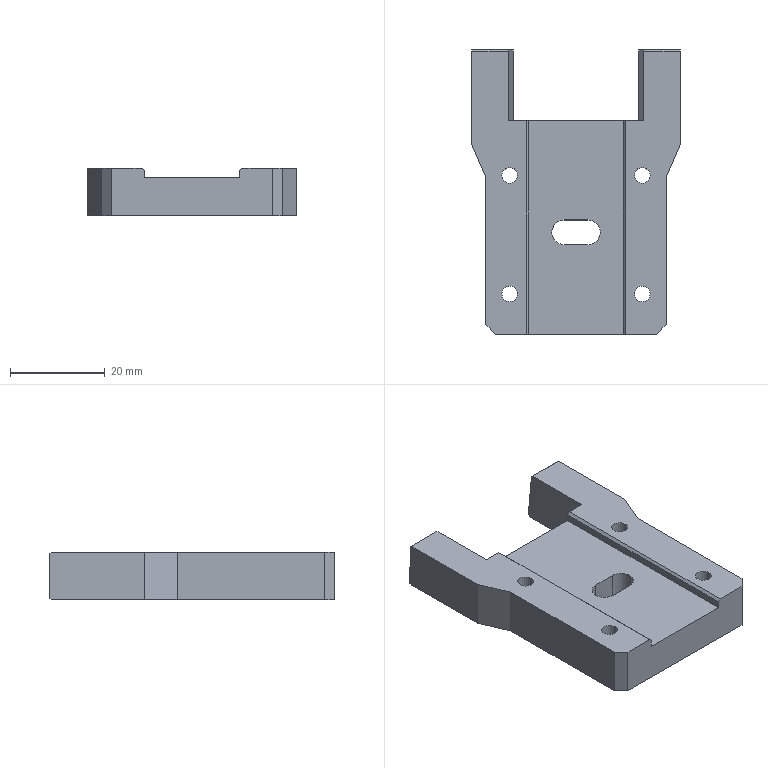Part | SolidWorks | features ICE 5, Chamfer 3, HoleWzd 3, Extrusion 1 | 1 solid | 51 faces | box 44 x 60 x 10 mm | volume 17311 mm3 | plane 28 | cylinder 17 | cone 6 | commonest cylinder face diameters 3.3 x12 5.2 x3 2.5 x2
STEP:
#1=CARTESIAN_POINT('',(-2.5,-5.9,8.));
#2=VERTEX_POINT('',#1);
#3=CARTESIAN_POINT('',(-5.1,-8.5,8.));
#4=VERTEX_POINT('',#3);
#5=CARTESIAN_POINT('',(-2.5,-8.5,8.));
#6=DIRECTION('',(0.,0.,1.));
#7=DIRECTION('',(1.,0.,0.));
#8=AXIS2_PLACEMENT_3D('',#5,#6,#7);
#9=CIRCLE('',#8,2.6);
#10=EDGE_CURVE('',#2,#4,#9,.T.);
#11=ORIENTED_EDGE('',*,*,#10,.T.);
#12=CARTESIAN_POINT('',(-5.1,-8.5,0.));
#13=VERTEX_POINT('',#12);
#14=CARTESIAN_POINT('',(-5.1,-8.5,10.));
#15=DIRECTION('',(0.,0.,-1.));
#16=VECTOR('',#15,1000.);
#17=LINE('',#14,#16);
#18=EDGE_CURVE('',#4,#13,#17,.T.);
#19=ORIENTED_EDGE('',*,*,#18,.T.);
#20=CARTESIAN_POINT('',(-2.5,-5.9,0.));
#21=VERTEX_POINT('',#20);
#22=CARTESIAN_POINT('',(-2.5,-8.5,0.));
#23=DIRECTION('',(0.,0.,-1.));
#24=DIRECTION('',(-1.,0.,0.));
#25=AXIS2_PLACEMENT_3D('',#22,#23,#24);
#26=CIRCLE('',#25,2.6);
#27=EDGE_CURVE('',#13,#21,#26,.T.);
#28=ORIENTED_EDGE('',*,*,#27,.T.);
#29=CARTESIAN_POINT('',(-2.5,-5.9,10.));
#30=DIRECTION('',(0.,0.,-1.));
#31=VECTOR('',#30,1000.);
#32=LINE('',#29,#31);
#33=EDGE_CURVE('',#2,#21,#32,.T.);
#34=ORIENTED_EDGE('',*,*,#33,.F.);
#35=EDGE_LOOP('',(#11,#19,#28,#34));
#36=FACE_OUTER_BOUND('',#35,.T.);
#37=CARTESIAN_POINT('',(-2.5,-8.5,10.));
#38=DIRECTION('',(0.,0.,-1.));
#39=DIRECTION('',(-1.,0.,0.));
#40=AXIS2_PLACEMENT_3D('',#37,#38,#39);
#41=CYLINDRICAL_SURFACE('',#40,2.6);
#42=ADVANCED_FACE('',(#36),#41,.F.);
#43=CARTESIAN_POINT('',(14.5,-15.,5.25));
#44=VERTEX_POINT('',#43);
#45=CARTESIAN_POINT('',(14.5,-15.,2.75));
#46=VERTEX_POINT('',#45);
#47=CARTESIAN_POINT('',(14.5,-15.,4.));
#48=DIRECTION('',(1.,0.,0.));
#49=DIRECTION('',(0.,0.,-1.));
#50=AXIS2_PLACEMENT_3D('',#47,#48,#49);
#51=CIRCLE('',#50,1.25);
#52=EDGE_CURVE('',#44,#46,#51,.T.);
#53=ORIENTED_EDGE('',*,*,#52,.F.);
#54=CARTESIAN_POINT('',(19.,-15.,5.25));
#55=VERTEX_POINT('',#54);
#56=CARTESIAN_POINT('',(22.,-15.,5.25));
#57=DIRECTION('',(1.,0.,0.));
#58=VECTOR('',#57,1000.);
#59=LINE('',#56,#58);
#60=EDGE_CURVE('',#44,#55,#59,.T.);
#61=ORIENTED_EDGE('',*,*,#60,.T.);
#62=CARTESIAN_POINT('',(19.,-15.,2.75));
#63=VERTEX_POINT('',#62);
#64=CARTESIAN_POINT('',(19.,-15.,4.));
#65=DIRECTION('',(1.,0.,0.));
#66=DIRECTION('',(0.,-1.,0.));
#67=AXIS2_PLACEMENT_3D('',#64,#65,#66);
#68=CIRCLE('',#67,1.25);
#69=EDGE_CURVE('',#55,#63,#68,.T.);
#70=ORIENTED_EDGE('',*,*,#69,.T.);
#71=CARTESIAN_POINT('',(22.,-15.,2.75));
#72=DIRECTION('',(1.,0.,0.));
#73=VECTOR('',#72,1000.);
#74=LINE('',#71,#73);
#75=EDGE_CURVE('',#46,#63,#74,.T.);
#76=ORIENTED_EDGE('',*,*,#75,.F.);
#77=EDGE_LOOP('',(#53,#61,#70,#76));
#78=FACE_OUTER_BOUND('',#77,.T.);
#79=CARTESIAN_POINT('',(22.,-15.,4.));
#80=DIRECTION('',(1.,0.,0.));
#81=DIRECTION('',(0.,0.,-1.));
#82=AXIS2_PLACEMENT_3D('',#79,#80,#81);
#83=CYLINDRICAL_SURFACE('',#82,1.25);
#84=ADVANCED_FACE('',(#78),#83,.F.);
#85=CARTESIAN_POINT('',(13.749,-15.,4.));
#86=VERTEX_POINT('',#85);
#87=CARTESIAN_POINT('',(14.5,-15.,2.75));
#88=DIRECTION('',(0.515,0.,-0.8572));
#89=VECTOR('',#88,1000.);
#90=LINE('',#87,#89);
#91=EDGE_CURVE('',#86,#46,#90,.T.);
#92=ORIENTED_EDGE('',*,*,#91,.F.);
#93=CARTESIAN_POINT('',(14.5,-15.,5.25));
#94=DIRECTION('',(0.515,0.,0.8572));
#95=VECTOR('',#94,1000.);
#96=LINE('',#93,#95);
#97=EDGE_CURVE('',#86,#44,#96,.T.);
#98=ORIENTED_EDGE('',*,*,#97,.T.);
#99=ORIENTED_EDGE('',*,*,#52,.T.);
#100=EDGE_LOOP('',(#92,#98,#99));
#101=FACE_OUTER_BOUND('',#100,.T.);
#102=CARTESIAN_POINT('',(14.5,-15.,4.));
#103=DIRECTION('',(1.,0.,0.));
#104=DIRECTION('',(0.,0.,-1.));
#105=AXIS2_PLACEMENT_3D('',#102,#103,#104);
#106=CONICAL_SURFACE('',#105,1.25,1.03);
#107=ADVANCED_FACE('',(#101),#106,.F.);
#108=CARTESIAN_POINT('',(-12.35,-21.5,0.));
#109=VERTEX_POINT('',#108);
#110=CARTESIAN_POINT('',(-15.65,-21.5,0.));
#111=VERTEX_POINT('',#110);
#112=CARTESIAN_POINT('',(-14.,-21.5,0.));
#113=DIRECTION('',(0.,0.,-1.));
#114=DIRECTION('',(-1.,0.,0.));
#115=AXIS2_PLACEMENT_3D('',#112,#113,#114);
#116=CIRCLE('',#115,1.65);
#117=EDGE_CURVE('',#109,#111,#116,.T.);
#118=ORIENTED_EDGE('',*,*,#117,.T.);
#119=CARTESIAN_POINT('',(-15.65,-21.5,10.));
#120=VERTEX_POINT('',#119);
#121=CARTESIAN_POINT('',(-15.65,-21.5,10.));
#122=DIRECTION('',(0.,0.,1.));
#123=VECTOR('',#122,1000.);
#124=LINE('',#121,#123);
#125=EDGE_CURVE('',#111,#120,#124,.T.);
#126=ORIENTED_EDGE('',*,*,#125,.T.);
#127=CARTESIAN_POINT('',(-12.35,-21.5,10.));
#128=VERTEX_POINT('',#127);
#129=CARTESIAN_POINT('',(-14.,-21.5,10.));
#130=DIRECTION('',(0.,0.,1.));
#131=DIRECTION('',(1.,0.,0.));
#132=AXIS2_PLACEMENT_3D('',#129,#130,#131);
#133=CIRCLE('',#132,1.65);
#134=EDGE_CURVE('',#120,#128,#133,.T.);
#135=ORIENTED_EDGE('',*,*,#134,.T.);
#136=CARTESIAN_POINT('',(-12.35,-21.5,10.));
#137=DIRECTION('',(0.,0.,1.));
#138=VECTOR('',#137,1000.);
#139=LINE('',#136,#138);
#140=EDGE_CURVE('',#109,#128,#139,.T.);
#141=ORIENTED_EDGE('',*,*,#140,.F.);
#142=EDGE_LOOP('',(#118,#126,#135,#141));
#143=FACE_OUTER_BOUND('',#142,.T.);
#144=CARTESIAN_POINT('',(-14.,-21.5,10.));
#145=DIRECTION('',(0.,0.,1.));
#146=DIRECTION('',(1.,0.,0.));
#147=AXIS2_PLACEMENT_3D('',#144,#145,#146);
#148=CYLINDRICAL_SURFACE('',#147,1.65);
#149=ADVANCED_FACE('',(#143),#148,.F.);
#150=CARTESIAN_POINT('',(15.65,-21.5,0.));
#151=VERTEX_POINT('',#150);
#152=CARTESIAN_POINT('',(12.35,-21.5,0.));
#153=VERTEX_POINT('',#152);
#154=CARTESIAN_POINT('',(14.,-21.5,0.));
#155=DIRECTION('',(0.,0.,-1.));
#156=DIRECTION('',(-1.,0.,0.));
#157=AXIS2_PLACEMENT_3D('',#154,#155,#156);
#158=CIRCLE('',#157,1.65);
#159=EDGE_CURVE('',#151,#153,#158,.T.);
#160=ORIENTED_EDGE('',*,*,#159,.T.);
#161=CARTESIAN_POINT('',(12.35,-21.5,10.));
#162=VERTEX_POINT('',#161);
#163=CARTESIAN_POINT('',(12.35,-21.5,10.));
#164=DIRECTION('',(0.,0.,1.));
#165=VECTOR('',#164,1000.);
#166=LINE('',#163,#165);
#167=EDGE_CURVE('',#153,#162,#166,.T.);
#168=ORIENTED_EDGE('',*,*,#167,.T.);
#169=CARTESIAN_POINT('',(15.65,-21.5,10.));
#170=VERTEX_POINT('',#169);
#171=CARTESIAN_POINT('',(14.,-21.5,10.));
#172=DIRECTION('',(0.,0.,1.));
#173=DIRECTION('',(1.,0.,0.));
#174=AXIS2_PLACEMENT_3D('',#171,#172,#173);
#175=CIRCLE('',#174,1.65);
#176=EDGE_CURVE('',#162,#170,#175,.T.);
#177=ORIENTED_EDGE('',*,*,#176,.T.);
#178=CARTESIAN_POINT('',(15.65,-21.5,10.));
#179=DIRECTION('',(0.,0.,1.));
#180=VECTOR('',#179,1000.);
#181=LINE('',#178,#180);
#182=EDGE_CURVE('',#151,#170,#181,.T.);
#183=ORIENTED_EDGE('',*,*,#182,.F.);
#184=EDGE_LOOP('',(#160,#168,#177,#183));
#185=FACE_OUTER_BOUND('',#184,.T.);
#186=CARTESIAN_POINT('',(14.,-21.5,10.));
#187=DIRECTION('',(0.,0.,1.));
#188=DIRECTION('',(1.,0.,0.));
#189=AXIS2_PLACEMENT_3D('',#186,#187,#188);
#190=CYLINDRICAL_SURFACE('',#189,1.65);
#191=ADVANCED_FACE('',(#185),#190,.F.);
#192=CARTESIAN_POINT('',(-12.35,3.5,0.));
#193=VERTEX_POINT('',#192);
#194=CARTESIAN_POINT('',(-15.65,3.5,0.));
#195=VERTEX_POINT('',#194);
#196=CARTESIAN_POINT('',(-14.,3.5,0.));
#197=DIRECTION('',(0.,0.,-1.));
#198=DIRECTION('',(-1.,0.,0.));
#199=AXIS2_PLACEMENT_3D('',#196,#197,#198);
#200=CIRCLE('',#199,1.65);
#201=EDGE_CURVE('',#193,#195,#200,.T.);
#202=ORIENTED_EDGE('',*,*,#201,.T.);
#203=CARTESIAN_POINT('',(-15.65,3.5,10.));
#204=VERTEX_POINT('',#203);
#205=CARTESIAN_POINT('',(-15.65,3.5,10.));
#206=DIRECTION('',(0.,0.,1.));
#207=VECTOR('',#206,1000.);
#208=LINE('',#205,#207);
#209=EDGE_CURVE('',#195,#204,#208,.T.);
#210=ORIENTED_EDGE('',*,*,#209,.T.);
#211=CARTESIAN_POINT('',(-12.35,3.5,10.));
#212=VERTEX_POINT('',#211);
#213=CARTESIAN_POINT('',(-14.,3.5,10.));
#214=DIRECTION('',(0.,0.,1.));
#215=DIRECTION('',(1.,0.,0.));
#216=AXIS2_PLACEMENT_3D('',#213,#214,#215);
#217=CIRCLE('',#216,1.65);
#218=EDGE_CURVE('',#204,#212,#217,.T.);
#219=ORIENTED_EDGE('',*,*,#218,.T.);
#220=CARTESIAN_POINT('',(-12.35,3.5,10.));
#221=DIRECTION('',(0.,0.,1.));
#222=VECTOR('',#221,1000.);
#223=LINE('',#220,#222);
#224=EDGE_CURVE('',#193,#212,#223,.T.);
#225=ORIENTED_EDGE('',*,*,#224,.F.);
#226=EDGE_LOOP('',(#202,#210,#219,#225));
#227=FACE_OUTER_BOUND('',#226,.T.);
#228=CARTESIAN_POINT('',(-14.,3.5,10.));
#229=DIRECTION('',(0.,0.,1.));
#230=DIRECTION('',(1.,0.,0.));
#231=AXIS2_PLACEMENT_3D('',#228,#229,#230);
#232=CYLINDRICAL_SURFACE('',#231,1.65);
#233=ADVANCED_FACE('',(#227),#232,.F.);
#234=CARTESIAN_POINT('',(15.65,3.5,0.));
#235=VERTEX_POINT('',#234);
#236=CARTESIAN_POINT('',(12.35,3.5,0.));
#237=VERTEX_POINT('',#236);
#238=CARTESIAN_POINT('',(14.,3.5,0.));
#239=DIRECTION('',(0.,0.,-1.));
#240=DIRECTION('',(-1.,0.,0.));
#241=AXIS2_PLACEMENT_3D('',#238,#239,#240);
#242=CIRCLE('',#241,1.65);
#243=EDGE_CURVE('',#235,#237,#242,.T.);
#244=ORIENTED_EDGE('',*,*,#243,.T.);
#245=CARTESIAN_POINT('',(12.35,3.5,10.));
#246=VERTEX_POINT('',#245);
#247=CARTESIAN_POINT('',(12.35,3.5,10.));
#248=DIRECTION('',(0.,0.,1.));
#249=VECTOR('',#248,1000.);
#250=LINE('',#247,#249);
#251=EDGE_CURVE('',#237,#246,#250,.T.);
#252=ORIENTED_EDGE('',*,*,#251,.T.);
#253=CARTESIAN_POINT('',(15.65,3.5,10.));
#254=VERTEX_POINT('',#253);
#255=CARTESIAN_POINT('',(14.,3.5,10.));
#256=DIRECTION('',(0.,0.,1.));
#257=DIRECTION('',(1.,0.,0.));
#258=AXIS2_PLACEMENT_3D('',#255,#256,#257);
#259=CIRCLE('',#258,1.65);
#260=EDGE_CURVE('',#246,#254,#259,.T.);
#261=ORIENTED_EDGE('',*,*,#260,.T.);
#262=CARTESIAN_POINT('',(15.65,3.5,10.));
#263=DIRECTION('',(0.,0.,1.));
#264=VECTOR('',#263,1000.);
#265=LINE('',#262,#264);
#266=EDGE_CURVE('',#235,#254,#265,.T.);
#267=ORIENTED_EDGE('',*,*,#266,.F.);
#268=EDGE_LOOP('',(#244,#252,#261,#267));
#269=FACE_OUTER_BOUND('',#268,.T.);
#270=CARTESIAN_POINT('',(14.,3.5,10.));
#271=DIRECTION('',(0.,0.,1.));
#272=DIRECTION('',(1.,0.,0.));
#273=AXIS2_PLACEMENT_3D('',#270,#271,#272);
#274=CYLINDRICAL_SURFACE('',#273,1.65);
#275=ADVANCED_FACE('',(#269),#274,.F.);
#276=CARTESIAN_POINT('',(-17.,19.9,3.35));
#277=VERTEX_POINT('',#276);
#278=CARTESIAN_POINT('',(-17.,19.9,6.65));
#279=VERTEX_POINT('',#278);
#280=CARTESIAN_POINT('',(-17.,19.9,5.));
#281=DIRECTION('',(0.,1.,0.));
#282=DIRECTION('',(0.,0.,1.));
#283=AXIS2_PLACEMENT_3D('',#280,#281,#282);
#284=CIRCLE('',#283,1.65);
#285=EDGE_CURVE('',#277,#279,#284,.T.);
#286=ORIENTED_EDGE('',*,*,#285,.F.);
#287=CARTESIAN_POINT('',(-17.,30.,3.35));
#288=VERTEX_POINT('',#287);
#289=CARTESIAN_POINT('',(-17.,30.,3.35));
#290=DIRECTION('',(0.,1.,0.));
#291=VECTOR('',#290,1000.);
#292=LINE('',#289,#291);
#293=EDGE_CURVE('',#277,#288,#292,.T.);
#294=ORIENTED_EDGE('',*,*,#293,.T.);
#295=CARTESIAN_POINT('',(-17.,30.,6.65));
#296=VERTEX_POINT('',#295);
#297=CARTESIAN_POINT('',(-17.,30.,5.));
#298=DIRECTION('',(0.,1.,0.));
#299=DIRECTION('',(0.,0.,1.));
#300=AXIS2_PLACEMENT_3D('',#297,#298,#299);
#301=CIRCLE('',#300,1.65);
#302=EDGE_CURVE('',#288,#296,#301,.T.);
#303=ORIENTED_EDGE('',*,*,#302,.T.);
#304=CARTESIAN_POINT('',(-17.,30.,6.65));
#305=DIRECTION('',(0.,1.,0.));
#306=VECTOR('',#305,1000.);
#307=LINE('',#304,#306);
#308=EDGE_CURVE('',#279,#296,#307,.T.);
#309=ORIENTED_EDGE('',*,*,#308,.F.);
#310=EDGE_LOOP('',(#286,#294,#303,#309));
#311=FACE_OUTER_BOUND('',#310,.T.);
#312=CARTESIAN_POINT('',(-17.,30.,5.));
#313=DIRECTION('',(0.,1.,0.));
#314=DIRECTION('',(0.,0.,1.));
#315=AXIS2_PLACEMENT_3D('',#312,#313,#314);
#316=CYLINDRICAL_SURFACE('',#315,1.65);
#317=ADVANCED_FACE('',(#311),#316,.F.);
#318=CARTESIAN_POINT('',(-17.,18.909,5.));
#319=VERTEX_POINT('',#318);
#320=CARTESIAN_POINT('',(-17.,19.9,6.65));
#321=DIRECTION('',(0.,0.515,0.8572));
#322=VECTOR('',#321,1000.);
#323=LINE('',#320,#322);
#324=EDGE_CURVE('',#319,#279,#323,.T.);
#325=ORIENTED_EDGE('',*,*,#324,.F.);
#326=CARTESIAN_POINT('',(-17.,19.9,3.35));
#327=DIRECTION('',(0.,0.515,-0.8572));
#328=VECTOR('',#327,1000.);
#329=LINE('',#326,#328);
#330=EDGE_CURVE('',#319,#277,#329,.T.);
#331=ORIENTED_EDGE('',*,*,#330,.T.);
#332=ORIENTED_EDGE('',*,*,#285,.T.);
#333=EDGE_LOOP('',(#325,#331,#332));
#334=FACE_OUTER_BOUND('',#333,.T.);
#335=CARTESIAN_POINT('',(-17.,19.9,5.));
#336=DIRECTION('',(0.,1.,0.));
#337=DIRECTION('',(0.,0.,1.));
#338=AXIS2_PLACEMENT_3D('',#335,#336,#337);
#339=CONICAL_SURFACE('',#338,1.65,1.03);
#340=ADVANCED_FACE('',(#334),#339,.F.);
#341=CARTESIAN_POINT('',(17.,19.9,3.35));
#342=VERTEX_POINT('',#341);
#343=CARTESIAN_POINT('',(17.,19.9,6.65));
#344=VERTEX_POINT('',#343);
#345=CARTESIAN_POINT('',(17.,19.9,5.));
#346=DIRECTION('',(0.,1.,0.));
#347=DIRECTION('',(0.,0.,1.));
#348=AXIS2_PLACEMENT_3D('',#345,#346,#347);
#349=CIRCLE('',#348,1.65);
#350=EDGE_CURVE('',#342,#344,#349,.T.);
#351=ORIENTED_EDGE('',*,*,#350,.F.);
#352=CARTESIAN_POINT('',(17.,30.,3.35));
#353=VERTEX_POINT('',#352);
#354=CARTESIAN_POINT('',(17.,30.,3.35));
#355=DIRECTION('',(0.,1.,0.));
#356=VECTOR('',#355,1000.);
#357=LINE('',#354,#356);
#358=EDGE_CURVE('',#342,#353,#357,.T.);
#359=ORIENTED_EDGE('',*,*,#358,.T.);
#360=CARTESIAN_POINT('',(17.,30.,6.65));
#361=VERTEX_POINT('',#360);
#362=CARTESIAN_POINT('',(17.,30.,5.));
#363=DIRECTION('',(0.,1.,0.));
#364=DIRECTION('',(0.,0.,1.));
#365=AXIS2_PLACEMENT_3D('',#362,#363,#364);
#366=CIRCLE('',#365,1.65);
#367=EDGE_CURVE('',#353,#361,#366,.T.);
#368=ORIENTED_EDGE('',*,*,#367,.T.);
#369=CARTESIAN_POINT('',(17.,30.,6.65));
#370=DIRECTION('',(0.,1.,0.));
#371=VECTOR('',#370,1000.);
#372=LINE('',#369,#371);
#373=EDGE_CURVE('',#344,#361,#372,.T.);
#374=ORIENTED_EDGE('',*,*,#373,.F.);
#375=EDGE_LOOP('',(#351,#359,#368,#374));
#376=FACE_OUTER_BOUND('',#375,.T.);
#377=CARTESIAN_POINT('',(17.,30.,5.));
#378=DIRECTION('',(0.,1.,0.));
#379=DIRECTION('',(0.,0.,1.));
#380=AXIS2_PLACEMENT_3D('',#377,#378,#379);
#381=CYLINDRICAL_SURFACE('',#380,1.65);
#382=ADVANCED_FACE('',(#376),#381,.F.);
#383=CARTESIAN_POINT('',(17.,18.909,5.));
#384=VERTEX_POINT('',#383);
#385=CARTESIAN_POINT('',(17.,19.9,6.65));
#386=DIRECTION('',(0.,0.515,0.8572));
#387=VECTOR('',#386,1000.);
#388=LINE('',#385,#387);
#389=EDGE_CURVE('',#384,#344,#388,.T.);
#390=ORIENTED_EDGE('',*,*,#389,.F.);
#391=CARTESIAN_POINT('',(17.,19.9,3.35));
#392=DIRECTION('',(0.,0.515,-0.8572));
#393=VECTOR('',#392,1000.);
#394=LINE('',#391,#393);
#395=EDGE_CURVE('',#384,#342,#394,.T.);
#396=ORIENTED_EDGE('',*,*,#395,.T.);
#397=ORIENTED_EDGE('',*,*,#350,.T.);
#398=EDGE_LOOP('',(#390,#396,#397));
#399=FACE_OUTER_BOUND('',#398,.T.);
#400=CARTESIAN_POINT('',(17.,19.9,5.));
#401=DIRECTION('',(0.,1.,0.));
#402=DIRECTION('',(0.,0.,1.));
#403=AXIS2_PLACEMENT_3D('',#400,#401,#402);
#404=CONICAL_SURFACE('',#403,1.65,1.03);
#405=ADVANCED_FACE('',(#399),#404,.F.);
#406=CARTESIAN_POINT('',(-14.,-21.5,10.));
#407=DIRECTION('',(0.,0.,1.));
#408=DIRECTION('',(1.,0.,0.));
#409=AXIS2_PLACEMENT_3D('',#406,#407,#408);
#410=CIRCLE('',#409,1.65);
#411=EDGE_CURVE('',#128,#120,#410,.T.);
#412=ORIENTED_EDGE('',*,*,#411,.F.);
#413=ORIENTED_EDGE('',*,*,#134,.F.);
#414=EDGE_LOOP('',(#412,#413));
#415=FACE_BOUND('',#414,.T.);
#416=CARTESIAN_POINT('',(-14.,3.5,10.));
#417=DIRECTION('',(0.,0.,1.));
#418=DIRECTION('',(1.,0.,0.));
#419=AXIS2_PLACEMENT_3D('',#416,#417,#418);
#420=CIRCLE('',#419,1.65);
#421=EDGE_CURVE('',#212,#204,#420,.T.);
#422=ORIENTED_EDGE('',*,*,#421,.F.);
#423=ORIENTED_EDGE('',*,*,#218,.F.);
#424=EDGE_LOOP('',(#422,#423));
#425=FACE_BOUND('',#424,.T.);
#426=CARTESIAN_POINT('',(-19.,-28.,10.));
#427=VERTEX_POINT('',#426);
#428=CARTESIAN_POINT('',(-19.,3.,10.));
#429=VERTEX_POINT('',#428);
#430=CARTESIAN_POINT('',(-19.,-30.,10.));
#431=DIRECTION('',(0.,1.,0.));
#432=VECTOR('',#431,1000.);
#433=LINE('',#430,#432);
#434=EDGE_CURVE('',#427,#429,#433,.T.);
#435=ORIENTED_EDGE('',*,*,#434,.F.);
#436=CARTESIAN_POINT('',(-17.,-30.,10.));
#437=VERTEX_POINT('',#436);
#438=CARTESIAN_POINT('',(-19.,-28.,10.));
#439=DIRECTION('',(0.7071,-0.7071,0.));
#440=VECTOR('',#439,1000.);
#441=LINE('',#438,#440);
#442=EDGE_CURVE('',#427,#437,#441,.T.);
#443=ORIENTED_EDGE('',*,*,#442,.T.);
#444=CARTESIAN_POINT('',(-10.5,-30.,10.));
#445=VERTEX_POINT('',#444);
#446=CARTESIAN_POINT('',(-22.,-30.,10.));
#447=DIRECTION('',(1.,0.,0.));
#448=VECTOR('',#447,1000.);
#449=LINE('',#446,#448);
#450=EDGE_CURVE('',#437,#445,#449,.T.);
#451=ORIENTED_EDGE('',*,*,#450,.T.);
#452=CARTESIAN_POINT('',(-10.5,15.,10.));
#453=VERTEX_POINT('',#452);
#454=CARTESIAN_POINT('',(-10.5,0.,10.));
#455=DIRECTION('',(0.,1.,0.));
#456=VECTOR('',#455,1000.);
#457=LINE('',#454,#456);
#458=EDGE_CURVE('',#445,#453,#457,.T.);
#459=ORIENTED_EDGE('',*,*,#458,.T.);
#460=CARTESIAN_POINT('',(-14.25,15.,10.));
#461=VERTEX_POINT('',#460);
#462=CARTESIAN_POINT('',(14.25,15.,10.));
#463=DIRECTION('',(1.,0.,0.));
#464=VECTOR('',#463,1000.);
#465=LINE('',#462,#464);
#466=EDGE_CURVE('',#461,#453,#465,.T.);
#467=ORIENTED_EDGE('',*,*,#466,.F.);
#468=CARTESIAN_POINT('',(-14.25,29.7,10.));
#469=VERTEX_POINT('',#468);
#470=CARTESIAN_POINT('',(-14.25,15.,10.));
#471=DIRECTION('',(0.,1.,0.));
#472=VECTOR('',#471,1000.);
#473=LINE('',#470,#472);
#474=EDGE_CURVE('',#461,#469,#473,.T.);
#475=ORIENTED_EDGE('',*,*,#474,.T.);
#476=CARTESIAN_POINT('',(-22.,29.7,10.));
#477=VERTEX_POINT('',#476);
#478=CARTESIAN_POINT('',(0.,29.7,10.));
#479=DIRECTION('',(-1.,0.,0.));
#480=VECTOR('',#479,1000.);
#481=LINE('',#478,#480);
#482=EDGE_CURVE('',#469,#477,#481,.T.);
#483=ORIENTED_EDGE('',*,*,#482,.T.);
#484=CARTESIAN_POINT('',(-22.,10.,10.));
#485=VERTEX_POINT('',#484);
#486=CARTESIAN_POINT('',(-22.,-30.,10.));
#487=DIRECTION('',(0.,-1.,0.));
#488=VECTOR('',#487,1000.);
#489=LINE('',#486,#488);
#490=EDGE_CURVE('',#477,#485,#489,.T.);
#491=ORIENTED_EDGE('',*,*,#490,.T.);
#492=CARTESIAN_POINT('',(-19.,3.,10.));
#493=DIRECTION('',(-0.3939,0.9191,0.));
#494=VECTOR('',#493,1000.);
#495=LINE('',#492,#494);
#496=EDGE_CURVE('',#429,#485,#495,.T.);
#497=ORIENTED_EDGE('',*,*,#496,.F.);
#498=EDGE_LOOP('',(#435,#443,#451,#459,#467,#475,#483,#491,#497));
#499=FACE_OUTER_BOUND('',#498,.T.);
#500=CARTESIAN_POINT('',(0.,0.,10.));
#501=DIRECTION('',(0.,0.,-1.));
#502=DIRECTION('',(-1.,0.,0.));
#503=AXIS2_PLACEMENT_3D('',#500,#501,#502);
#504=PLANE('',#503);
#505=ADVANCED_FACE('',(#415,#425,#499),#504,.F.);
#506=CARTESIAN_POINT('',(17.,30.,5.));
#507=DIRECTION('',(0.,1.,0.));
#508=DIRECTION('',(0.,0.,1.));
#509=AXIS2_PLACEMENT_3D('',#506,#507,#508);
#510=CIRCLE('',#509,1.65);
#511=EDGE_CURVE('',#361,#353,#510,.T.);
#512=ORIENTED_EDGE('',*,*,#511,.F.);
#513=ORIENTED_EDGE('',*,*,#367,.F.);
#514=EDGE_LOOP('',(#512,#513));
#515=FACE_BOUND('',#514,.T.);
#516=CARTESIAN_POINT('',(14.22,30.,9.7));
#517=VERTEX_POINT('',#516);
#518=CARTESIAN_POINT('',(13.28,30.,0.3));
#519=VERTEX_POINT('',#518);
#520=CARTESIAN_POINT('',(13.25,30.,0.));
#521=DIRECTION('',(-0.0995,0.,-0.995));
#522=VECTOR('',#521,1000.);
#523=LINE('',#520,#522);
#524=EDGE_CURVE('',#517,#519,#523,.T.);
#525=ORIENTED_EDGE('',*,*,#524,.F.);
#526=CARTESIAN_POINT('',(22.,30.,9.7));
#527=VERTEX_POINT('',#526);
#528=CARTESIAN_POINT('',(-22.,30.,9.7));
#529=DIRECTION('',(1.,0.,0.));
#530=VECTOR('',#529,1000.);
#531=LINE('',#528,#530);
#532=EDGE_CURVE('',#517,#527,#531,.T.);
#533=ORIENTED_EDGE('',*,*,#532,.T.);
#534=CARTESIAN_POINT('',(22.,30.,0.3));
#535=VERTEX_POINT('',#534);
#536=CARTESIAN_POINT('',(22.,30.,10.));
#537=DIRECTION('',(0.,0.,-1.));
#538=VECTOR('',#537,1000.);
#539=LINE('',#536,#538);
#540=EDGE_CURVE('',#527,#535,#539,.T.);
#541=ORIENTED_EDGE('',*,*,#540,.T.);
#542=CARTESIAN_POINT('',(13.25,30.,0.3));
#543=DIRECTION('',(-1.,0.,0.));
#544=VECTOR('',#543,1000.);
#545=LINE('',#542,#544);
#546=EDGE_CURVE('',#535,#519,#545,.T.);
#547=ORIENTED_EDGE('',*,*,#546,.T.);
#548=EDGE_LOOP('',(#525,#533,#541,#547));
#549=FACE_OUTER_BOUND('',#548,.T.);
#550=CARTESIAN_POINT('',(-22.,30.,10.));
#551=DIRECTION('',(0.,-1.,0.));
#552=DIRECTION('',(0.,0.,-1.));
#553=AXIS2_PLACEMENT_3D('',#550,#551,#552);
#554=PLANE('',#553);
#555=ADVANCED_FACE('',(#515,#549),#554,.F.);
#556=CARTESIAN_POINT('',(22.,10.,10.));
#557=VERTEX_POINT('',#556);
#558=CARTESIAN_POINT('',(22.,29.7,10.));
#559=VERTEX_POINT('',#558);
#560=CARTESIAN_POINT('',(22.,-30.,10.));
#561=DIRECTION('',(0.,1.,0.));
#562=VECTOR('',#561,1000.);
#563=LINE('',#560,#562);
#564=EDGE_CURVE('',#557,#559,#563,.T.);
#565=ORIENTED_EDGE('',*,*,#564,.F.);
#566=CARTESIAN_POINT('',(22.,10.,0.));
#567=VERTEX_POINT('',#566);
#568=CARTESIAN_POINT('',(22.,10.,0.));
#569=DIRECTION('',(0.,0.,1.));
#570=VECTOR('',#569,1000.);
#571=LINE('',#568,#570);
#572=EDGE_CURVE('',#567,#557,#571,.T.);
#573=ORIENTED_EDGE('',*,*,#572,.F.);
#574=CARTESIAN_POINT('',(22.,29.7,0.));
#575=VERTEX_POINT('',#574);
#576=CARTESIAN_POINT('',(22.,-30.,0.));
#577=DIRECTION('',(0.,1.,0.));
#578=VECTOR('',#577,1000.);
#579=LINE('',#576,#578);
#580=EDGE_CURVE('',#567,#575,#579,.T.);
#581=ORIENTED_EDGE('',*,*,#580,.T.);
#582=CARTESIAN_POINT('',(22.,30.,0.3));
#583=DIRECTION('',(0.,0.7071,0.7071));
#584=VECTOR('',#583,1000.);
#585=LINE('',#582,#584);
#586=EDGE_CURVE('',#575,#535,#585,.T.);
#587=ORIENTED_EDGE('',*,*,#586,.T.);
#588=ORIENTED_EDGE('',*,*,#540,.F.);
#589=CARTESIAN_POINT('',(22.,29.7,10.));
#590=DIRECTION('',(0.,-0.7071,0.7071));
#591=VECTOR('',#590,1000.);
#592=LINE('',#589,#591);
#593=EDGE_CURVE('',#527,#559,#592,.T.);
#594=ORIENTED_EDGE('',*,*,#593,.T.);
#595=EDGE_LOOP('',(#565,#573,#581,#587,#588,#594));
#596=FACE_OUTER_BOUND('',#595,.T.);
#597=CARTESIAN_POINT('',(22.,-30.,10.));
#598=DIRECTION('',(-1.,0.,0.));
#599=DIRECTION('',(0.,0.,1.));
#600=AXIS2_PLACEMENT_3D('',#597,#598,#599);
#601=PLANE('',#600);
#602=ADVANCED_FACE('',(#596),#601,.F.);
#603=CARTESIAN_POINT('',(-17.,30.,5.));
#604=DIRECTION('',(0.,1.,0.));
#605=DIRECTION('',(0.,0.,1.));
#606=AXIS2_PLACEMENT_3D('',#603,#604,#605);
#607=CIRCLE('',#606,1.65);
#608=EDGE_CURVE('',#296,#288,#607,.T.);
#609=ORIENTED_EDGE('',*,*,#608,.F.);
#610=ORIENTED_EDGE('',*,*,#302,.F.);
#611=EDGE_LOOP('',(#609,#610));
#612=FACE_BOUND('',#611,.T.);
#613=CARTESIAN_POINT('',(-13.28,30.,0.3));
#614=VERTEX_POINT('',#613);
#615=CARTESIAN_POINT('',(-14.22,30.,9.7));
#616=VERTEX_POINT('',#615);
#617=CARTESIAN_POINT('',(-14.25,30.,10.));
#618=DIRECTION('',(-0.0995,0.,0.995));
#619=VECTOR('',#618,1000.);
#620=LINE('',#617,#619);
#621=EDGE_CURVE('',#614,#616,#620,.T.);
#622=ORIENTED_EDGE('',*,*,#621,.F.);
#623=CARTESIAN_POINT('',(-22.,30.,0.3));
#624=VERTEX_POINT('',#623);
#625=CARTESIAN_POINT('',(-22.,30.,0.3));
#626=DIRECTION('',(-1.,0.,0.));
#627=VECTOR('',#626,1000.);
#628=LINE('',#625,#627);
#629=EDGE_CURVE('',#614,#624,#628,.T.);
#630=ORIENTED_EDGE('',*,*,#629,.T.);
#631=CARTESIAN_POINT('',(-22.,30.,9.7));
#632=VERTEX_POINT('',#631);
#633=CARTESIAN_POINT('',(-22.,30.,10.));
#634=DIRECTION('',(0.,0.,-1.));
#635=VECTOR('',#634,1000.);
#636=LINE('',#633,#635);
#637=EDGE_CURVE('',#632,#624,#636,.T.);
#638=ORIENTED_EDGE('',*,*,#637,.F.);
#639=CARTESIAN_POINT('',(-22.,30.,9.7));
#640=DIRECTION('',(1.,0.,0.));
#641=VECTOR('',#640,1000.);
#642=LINE('',#639,#641);
#643=EDGE_CURVE('',#632,#616,#642,.T.);
#644=ORIENTED_EDGE('',*,*,#643,.T.);
#645=EDGE_LOOP('',(#622,#630,#638,#644));
#646=FACE_OUTER_BOUND('',#645,.T.);
#647=CARTESIAN_POINT('',(-22.,30.,10.));
#648=DIRECTION('',(0.,-1.,0.));
#649=DIRECTION('',(0.,0.,-1.));
#650=AXIS2_PLACEMENT_3D('',#647,#648,#649);
#651=PLANE('',#650);
#652=ADVANCED_FACE('',(#612,#646),#651,.F.);
#653=CARTESIAN_POINT('',(-22.,29.7,0.));
#654=VERTEX_POINT('',#653);
#655=CARTESIAN_POINT('',(-22.,10.,0.));
#656=VERTEX_POINT('',#655);
#657=CARTESIAN_POINT('',(-22.,-30.,0.));
#658=DIRECTION('',(0.,-1.,0.));
#659=VECTOR('',#658,1000.);
#660=LINE('',#657,#659);
#661=EDGE_CURVE('',#654,#656,#660,.T.);
#662=ORIENTED_EDGE('',*,*,#661,.T.);
#663=CARTESIAN_POINT('',(-22.,10.,0.));
#664=DIRECTION('',(0.,0.,1.));
#665=VECTOR('',#664,1000.);
#666=LINE('',#663,#665);
#667=EDGE_CURVE('',#656,#485,#666,.T.);
#668=ORIENTED_EDGE('',*,*,#667,.T.);
#669=ORIENTED_EDGE('',*,*,#490,.F.);
#670=CARTESIAN_POINT('',(-22.,29.7,10.));
#671=DIRECTION('',(0.,0.7071,-0.7071));
#672=VECTOR('',#671,1000.);
#673=LINE('',#670,#672);
#674=EDGE_CURVE('',#477,#632,#673,.T.);
#675=ORIENTED_EDGE('',*,*,#674,.T.);
#676=ORIENTED_EDGE('',*,*,#637,.T.);
#677=CARTESIAN_POINT('',(-22.,30.,0.3));
#678=DIRECTION('',(0.,-0.7071,-0.7071));
#679=VECTOR('',#678,1000.);
#680=LINE('',#677,#679);
#681=EDGE_CURVE('',#624,#654,#680,.T.);
#682=ORIENTED_EDGE('',*,*,#681,.T.);
#683=EDGE_LOOP('',(#662,#668,#669,#675,#676,#682));
#684=FACE_OUTER_BOUND('',#683,.T.);
#685=CARTESIAN_POINT('',(-22.,-30.,10.));
#686=DIRECTION('',(1.,0.,0.));
#687=DIRECTION('',(0.,0.,-1.));
#688=AXIS2_PLACEMENT_3D('',#685,#686,#687);
#689=PLANE('',#688);
#690=ADVANCED_FACE('',(#684),#689,.F.);
#691=CARTESIAN_POINT('',(-17.,-30.,0.));
#692=VERTEX_POINT('',#691);
#693=CARTESIAN_POINT('',(17.,-30.,0.));
#694=VERTEX_POINT('',#693);
#695=CARTESIAN_POINT('',(-22.,-30.,0.));
#696=DIRECTION('',(1.,0.,0.));
#697=VECTOR('',#696,1000.);
#698=LINE('',#695,#697);
#699=EDGE_CURVE('',#692,#694,#698,.T.);
#700=ORIENTED_EDGE('',*,*,#699,.T.);
#701=CARTESIAN_POINT('',(17.,-30.,10.));
#702=VERTEX_POINT('',#701);
#703=CARTESIAN_POINT('',(17.,-30.,10.));
#704=DIRECTION('',(0.,0.,1.));
#705=VECTOR('',#704,1000.);
#706=LINE('',#703,#705);
#707=EDGE_CURVE('',#694,#702,#706,.T.);
#708=ORIENTED_EDGE('',*,*,#707,.T.);
#709=CARTESIAN_POINT('',(10.5,-30.,10.));
#710=VERTEX_POINT('',#709);
#711=CARTESIAN_POINT('',(-22.,-30.,10.));
#712=DIRECTION('',(1.,0.,0.));
#713=VECTOR('',#712,1000.);
#714=LINE('',#711,#713);
#715=EDGE_CURVE('',#710,#702,#714,.T.);
#716=ORIENTED_EDGE('',*,*,#715,.F.);
#717=CARTESIAN_POINT('',(10.,-30.,9.5));
#718=VERTEX_POINT('',#717);
#719=CARTESIAN_POINT('',(10.,-30.,9.5));
#720=DIRECTION('',(-0.7071,0.,-0.7071));
#721=VECTOR('',#720,1000.);
#722=LINE('',#719,#721);
#723=EDGE_CURVE('',#710,#718,#722,.T.);
#724=ORIENTED_EDGE('',*,*,#723,.T.);
#725=CARTESIAN_POINT('',(10.,-30.,8.));
#726=VERTEX_POINT('',#725);
#727=CARTESIAN_POINT('',(10.,-30.,8.));
#728=DIRECTION('',(0.,0.,1.));
#729=VECTOR('',#728,1000.);
#730=LINE('',#727,#729);
#731=EDGE_CURVE('',#726,#718,#730,.T.);
#732=ORIENTED_EDGE('',*,*,#731,.F.);
#733=CARTESIAN_POINT('',(-10.,-30.,8.));
#734=VERTEX_POINT('',#733);
#735=CARTESIAN_POINT('',(10.,-30.,8.));
#736=DIRECTION('',(1.,0.,0.));
#737=VECTOR('',#736,1000.);
#738=LINE('',#735,#737);
#739=EDGE_CURVE('',#734,#726,#738,.T.);
#740=ORIENTED_EDGE('',*,*,#739,.F.);
#741=CARTESIAN_POINT('',(-10.,-30.,9.5));
#742=VERTEX_POINT('',#741);
#743=CARTESIAN_POINT('',(-10.,-30.,8.));
#744=DIRECTION('',(0.,0.,1.));
#745=VECTOR('',#744,1000.);
#746=LINE('',#743,#745);
#747=EDGE_CURVE('',#734,#742,#746,.T.);
#748=ORIENTED_EDGE('',*,*,#747,.T.);
#749=CARTESIAN_POINT('',(-10.,-30.,9.5));
#750=DIRECTION('',(-0.7071,0.,0.7071));
#751=VECTOR('',#750,1000.);
#752=LINE('',#749,#751);
#753=EDGE_CURVE('',#742,#445,#752,.T.);
#754=ORIENTED_EDGE('',*,*,#753,.T.);
#755=ORIENTED_EDGE('',*,*,#450,.F.);
#756=CARTESIAN_POINT('',(-17.,-30.,10.));
#757=DIRECTION('',(0.,0.,-1.));
#758=VECTOR('',#757,1000.);
#759=LINE('',#756,#758);
#760=EDGE_CURVE('',#437,#692,#759,.T.);
#761=ORIENTED_EDGE('',*,*,#760,.T.);
#762=EDGE_LOOP('',(#700,#708,#716,#724,#732,#740,#748,#754,#755,#761));
#763=FACE_OUTER_BOUND('',#762,.T.);
#764=CARTESIAN_POINT('',(-22.,-30.,10.));
#765=DIRECTION('',(0.,1.,0.));
#766=DIRECTION('',(0.,0.,1.));
#767=AXIS2_PLACEMENT_3D('',#764,#765,#766);
#768=PLANE('',#767);
#769=ADVANCED_FACE('',(#763),#768,.F.);
#770=CARTESIAN_POINT('',(14.,-21.5,10.));
#771=DIRECTION('',(0.,0.,1.));
#772=DIRECTION('',(1.,0.,0.));
#773=AXIS2_PLACEMENT_3D('',#770,#771,#772);
#774=CIRCLE('',#773,1.65);
#775=EDGE_CURVE('',#170,#162,#774,.T.);
#776=ORIENTED_EDGE('',*,*,#775,.F.);
#777=ORIENTED_EDGE('',*,*,#176,.F.);
#778=EDGE_LOOP('',(#776,#777));
#779=FACE_BOUND('',#778,.T.);
#780=CARTESIAN_POINT('',(14.,3.5,10.));
#781=DIRECTION('',(0.,0.,1.));
#782=DIRECTION('',(1.,0.,0.));
#783=AXIS2_PLACEMENT_3D('',#780,#781,#782);
#784=CIRCLE('',#783,1.65);
#785=EDGE_CURVE('',#254,#246,#784,.T.);
#786=ORIENTED_EDGE('',*,*,#785,.F.);
#787=ORIENTED_EDGE('',*,*,#260,.F.);
#788=EDGE_LOOP('',(#786,#787));
#789=FACE_BOUND('',#788,.T.);
#790=ORIENTED_EDGE('',*,*,#715,.T.);
#791=CARTESIAN_POINT('',(19.,-28.,10.));
#792=VERTEX_POINT('',#791);
#793=CARTESIAN_POINT('',(17.,-30.,10.));
#794=DIRECTION('',(0.7071,0.7071,0.));
#795=VECTOR('',#794,1000.);
#796=LINE('',#793,#795);
#797=EDGE_CURVE('',#702,#792,#796,.T.);
#798=ORIENTED_EDGE('',*,*,#797,.T.);
#799=CARTESIAN_POINT('',(19.,3.,10.));
#800=VERTEX_POINT('',#799);
#801=CARTESIAN_POINT('',(19.,-30.,10.));
#802=DIRECTION('',(0.,-1.,0.));
#803=VECTOR('',#802,1000.);
#804=LINE('',#801,#803);
#805=EDGE_CURVE('',#800,#792,#804,.T.);
#806=ORIENTED_EDGE('',*,*,#805,.F.);
#807=CARTESIAN_POINT('',(19.,3.,10.));
#808=DIRECTION('',(-0.3939,-0.9191,0.));
#809=VECTOR('',#808,1000.);
#810=LINE('',#807,#809);
#811=EDGE_CURVE('',#557,#800,#810,.T.);
#812=ORIENTED_EDGE('',*,*,#811,.F.);
#813=ORIENTED_EDGE('',*,*,#564,.T.);
#814=CARTESIAN_POINT('',(14.25,29.7,10.));
#815=VERTEX_POINT('',#814);
#816=CARTESIAN_POINT('',(0.,29.7,10.));
#817=DIRECTION('',(-1.,0.,0.));
#818=VECTOR('',#817,1000.);
#819=LINE('',#816,#818);
#820=EDGE_CURVE('',#559,#815,#819,.T.);
#821=ORIENTED_EDGE('',*,*,#820,.T.);
#822=CARTESIAN_POINT('',(14.25,15.,10.));
#823=VERTEX_POINT('',#822);
#824=CARTESIAN_POINT('',(14.25,15.,10.));
#825=DIRECTION('',(0.,1.,0.));
#826=VECTOR('',#825,1000.);
#827=LINE('',#824,#826);
#828=EDGE_CURVE('',#823,#815,#827,.T.);
#829=ORIENTED_EDGE('',*,*,#828,.F.);
#830=CARTESIAN_POINT('',(10.5,15.,10.));
#831=VERTEX_POINT('',#830);
#832=CARTESIAN_POINT('',(14.25,15.,10.));
#833=DIRECTION('',(1.,0.,0.));
#834=VECTOR('',#833,1000.);
#835=LINE('',#832,#834);
#836=EDGE_CURVE('',#831,#823,#835,.T.);
#837=ORIENTED_EDGE('',*,*,#836,.F.);
#838=CARTESIAN_POINT('',(10.5,0.,10.));
#839=DIRECTION('',(0.,-1.,0.));
#840=VECTOR('',#839,1000.);
#841=LINE('',#838,#840);
#842=EDGE_CURVE('',#831,#710,#841,.T.);
#843=ORIENTED_EDGE('',*,*,#842,.T.);
#844=EDGE_LOOP('',(#790,#798,#806,#812,#813,#821,#829,#837,#843));
#845=FACE_OUTER_BOUND('',#844,.T.);
#846=CARTESIAN_POINT('',(0.,0.,10.));
#847=DIRECTION('',(0.,0.,-1.));
#848=DIRECTION('',(-1.,0.,0.));
#849=AXIS2_PLACEMENT_3D('',#846,#847,#848);
#850=PLANE('',#849);
#851=ADVANCED_FACE('',(#779,#789,#845),#850,.F.);
#852=CARTESIAN_POINT('',(2.5,-5.9,0.));
#853=VERTEX_POINT('',#852);
#854=CARTESIAN_POINT('',(2.5,-11.1,0.));
#855=VERTEX_POINT('',#854);
#856=CARTESIAN_POINT('',(2.5,-8.5,0.));
#857=DIRECTION('',(0.,0.,-1.));
#858=DIRECTION('',(-1.,0.,0.));
#859=AXIS2_PLACEMENT_3D('',#856,#857,#858);
#860=CIRCLE('',#859,2.6);
#861=EDGE_CURVE('',#853,#855,#860,.T.);
#862=ORIENTED_EDGE('',*,*,#861,.F.);
#863=CARTESIAN_POINT('',(2.5,-5.9,0.));
#864=DIRECTION('',(1.,0.,0.));
#865=VECTOR('',#864,1000.);
#866=LINE('',#863,#865);
#867=EDGE_CURVE('',#21,#853,#866,.T.);
#868=ORIENTED_EDGE('',*,*,#867,.F.);
#869=ORIENTED_EDGE('',*,*,#27,.F.);
#870=CARTESIAN_POINT('',(-2.5,-11.1,0.));
#871=VERTEX_POINT('',#870);
#872=CARTESIAN_POINT('',(-2.5,-8.5,0.));
#873=DIRECTION('',(0.,0.,-1.));
#874=DIRECTION('',(-1.,0.,0.));
#875=AXIS2_PLACEMENT_3D('',#872,#873,#874);
#876=CIRCLE('',#875,2.6);
#877=EDGE_CURVE('',#871,#13,#876,.T.);
#878=ORIENTED_EDGE('',*,*,#877,.F.);
#879=CARTESIAN_POINT('',(2.5,-11.1,0.));
#880=DIRECTION('',(-1.,0.,0.));
#881=VECTOR('',#880,1000.);
#882=LINE('',#879,#881);
#883=EDGE_CURVE('',#855,#871,#882,.T.);
#884=ORIENTED_EDGE('',*,*,#883,.F.);
#885=EDGE_LOOP('',(#862,#868,#869,#878,#884));
#886=FACE_BOUND('',#885,.T.);
#887=CARTESIAN_POINT('',(19.,3.,0.));
#888=VERTEX_POINT('',#887);
#889=CARTESIAN_POINT('',(19.,-28.,0.));
#890=VERTEX_POINT('',#889);
#891=CARTESIAN_POINT('',(19.,-30.,0.));
#892=DIRECTION('',(0.,-1.,0.));
#893=VECTOR('',#892,1000.);
#894=LINE('',#891,#893);
#895=EDGE_CURVE('',#888,#890,#894,.T.);
#896=ORIENTED_EDGE('',*,*,#895,.T.);
#897=CARTESIAN_POINT('',(23.5,-23.5,0.));
#898=DIRECTION('',(-0.7071,-0.7071,0.));
#899=VECTOR('',#898,1000.);
#900=LINE('',#897,#899);
#901=EDGE_CURVE('',#890,#694,#900,.T.);
#902=ORIENTED_EDGE('',*,*,#901,.T.);
#903=ORIENTED_EDGE('',*,*,#699,.F.);
#904=CARTESIAN_POINT('',(-19.,-28.,0.));
#905=VERTEX_POINT('',#904);
#906=CARTESIAN_POINT('',(-23.5,-23.5,0.));
#907=DIRECTION('',(-0.7071,0.7071,0.));
#908=VECTOR('',#907,1000.);
#909=LINE('',#906,#908);
#910=EDGE_CURVE('',#692,#905,#909,.T.);
#911=ORIENTED_EDGE('',*,*,#910,.T.);
#912=CARTESIAN_POINT('',(-19.,3.,0.));
#913=VERTEX_POINT('',#912);
#914=CARTESIAN_POINT('',(-19.,-30.,0.));
#915=DIRECTION('',(0.,1.,0.));
#916=VECTOR('',#915,1000.);
#917=LINE('',#914,#916);
#918=EDGE_CURVE('',#905,#913,#917,.T.);
#919=ORIENTED_EDGE('',*,*,#918,.T.);
#920=CARTESIAN_POINT('',(-19.,3.,0.));
#921=DIRECTION('',(-0.3939,0.9191,0.));
#922=VECTOR('',#921,1000.);
#923=LINE('',#920,#922);
#924=EDGE_CURVE('',#913,#656,#923,.T.);
#925=ORIENTED_EDGE('',*,*,#924,.T.);
#926=ORIENTED_EDGE('',*,*,#661,.F.);
#927=CARTESIAN_POINT('',(-13.25,29.7,0.));
#928=VERTEX_POINT('',#927);
#929=CARTESIAN_POINT('',(-13.25,29.7,0.));
#930=DIRECTION('',(1.,0.,0.));
#931=VECTOR('',#930,1000.);
#932=LINE('',#929,#931);
#933=EDGE_CURVE('',#654,#928,#932,.T.);
#934=ORIENTED_EDGE('',*,*,#933,.T.);
#935=CARTESIAN_POINT('',(-13.25,15.,0.));
#936=VERTEX_POINT('',#935);
#937=CARTESIAN_POINT('',(-13.25,15.,0.));
#938=DIRECTION('',(0.,1.,0.));
#939=VECTOR('',#938,1000.);
#940=LINE('',#937,#939);
#941=EDGE_CURVE('',#936,#928,#940,.T.);
#942=ORIENTED_EDGE('',*,*,#941,.F.);
#943=CARTESIAN_POINT('',(13.25,15.,0.));
#944=VERTEX_POINT('',#943);
#945=CARTESIAN_POINT('',(-13.25,15.,0.));
#946=DIRECTION('',(-1.,0.,0.));
#947=VECTOR('',#946,1000.);
#948=LINE('',#945,#947);
#949=EDGE_CURVE('',#944,#936,#948,.T.);
#950=ORIENTED_EDGE('',*,*,#949,.F.);
#951=CARTESIAN_POINT('',(13.25,29.7,0.));
#952=VERTEX_POINT('',#951);
#953=CARTESIAN_POINT('',(13.25,15.,0.));
#954=DIRECTION('',(0.,1.,0.));
#955=VECTOR('',#954,1000.);
#956=LINE('',#953,#955);
#957=EDGE_CURVE('',#944,#952,#956,.T.);
#958=ORIENTED_EDGE('',*,*,#957,.T.);
#959=CARTESIAN_POINT('',(22.,29.7,0.));
#960=DIRECTION('',(1.,0.,0.));
#961=VECTOR('',#960,1000.);
#962=LINE('',#959,#961);
#963=EDGE_CURVE('',#952,#575,#962,.T.);
#964=ORIENTED_EDGE('',*,*,#963,.T.);
#965=ORIENTED_EDGE('',*,*,#580,.F.);
#966=CARTESIAN_POINT('',(19.,3.,0.));
#967=DIRECTION('',(-0.3939,-0.9191,0.));
#968=VECTOR('',#967,1000.);
#969=LINE('',#966,#968);
#970=EDGE_CURVE('',#567,#888,#969,.T.);
#971=ORIENTED_EDGE('',*,*,#970,.T.);
#972=EDGE_LOOP('',(#896,#902,#903,#911,#919,#925,#926,#934,#942,#950,#958,#964,#965,#971));
#973=FACE_OUTER_BOUND('',#972,.T.);
#974=ORIENTED_EDGE('',*,*,#117,.F.);
#975=CARTESIAN_POINT('',(-14.,-21.5,0.));
#976=DIRECTION('',(0.,0.,-1.));
#977=DIRECTION('',(-1.,0.,0.));
#978=AXIS2_PLACEMENT_3D('',#975,#976,#977);
#979=CIRCLE('',#978,1.65);
#980=EDGE_CURVE('',#111,#109,#979,.T.);
#981=ORIENTED_EDGE('',*,*,#980,.F.);
#982=EDGE_LOOP('',(#974,#981));
#983=FACE_BOUND('',#982,.T.);
#984=ORIENTED_EDGE('',*,*,#159,.F.);
#985=CARTESIAN_POINT('',(14.,-21.5,0.));
#986=DIRECTION('',(0.,0.,-1.));
#987=DIRECTION('',(-1.,0.,0.));
#988=AXIS2_PLACEMENT_3D('',#985,#986,#987);
#989=CIRCLE('',#988,1.65);
#990=EDGE_CURVE('',#153,#151,#989,.T.);
#991=ORIENTED_EDGE('',*,*,#990,.F.);
#992=EDGE_LOOP('',(#984,#991));
#993=FACE_BOUND('',#992,.T.);
#994=ORIENTED_EDGE('',*,*,#201,.F.);
#995=CARTESIAN_POINT('',(-14.,3.5,0.));
#996=DIRECTION('',(0.,0.,-1.));
#997=DIRECTION('',(-1.,0.,0.));
#998=AXIS2_PLACEMENT_3D('',#995,#996,#997);
#999=CIRCLE('',#998,1.65);
#1000=EDGE_CURVE('',#195,#193,#999,.T.);
#1001=ORIENTED_EDGE('',*,*,#1000,.F.);
#1002=EDGE_LOOP('',(#994,#1001));
#1003=FACE_BOUND('',#1002,.T.);
#1004=ORIENTED_EDGE('',*,*,#243,.F.);
#1005=CARTESIAN_POINT('',(14.,3.5,0.));
#1006=DIRECTION('',(0.,0.,-1.));
#1007=DIRECTION('',(-1.,0.,0.));
#1008=AXIS2_PLACEMENT_3D('',#1005,#1006,#1007);
#1009=CIRCLE('',#1008,1.65);
#1010=EDGE_CURVE('',#237,#235,#1009,.T.);
#1011=ORIENTED_EDGE('',*,*,#1010,.F.);
#1012=EDGE_LOOP('',(#1004,#1011));
#1013=FACE_BOUND('',#1012,.T.);
#1014=CARTESIAN_POINT('',(0.,0.,0.));
#1015=DIRECTION('',(0.,0.,-1.));
#1016=DIRECTION('',(-1.,0.,0.));
#1017=AXIS2_PLACEMENT_3D('',#1014,#1015,#1016);
#1018=PLANE('',#1017);
#1019=ADVANCED_FACE('',(#886,#973,#983,#993,#1003,#1013),#1018,.T.);
#1020=ORIENTED_EDGE('',*,*,#828,.T.);
#1021=CARTESIAN_POINT('',(14.179,30.409,9.291));
#1022=DIRECTION('',(-0.07053,0.7053,-0.7053));
#1023=VECTOR('',#1022,1000.);
#1024=LINE('',#1021,#1023);
#1025=EDGE_CURVE('',#815,#517,#1024,.T.);
#1026=ORIENTED_EDGE('',*,*,#1025,.T.);
#1027=ORIENTED_EDGE('',*,*,#524,.T.);
#1028=CARTESIAN_POINT('',(13.104,28.245,-1.455));
#1029=DIRECTION('',(-0.07053,-0.7053,-0.7053));
#1030=VECTOR('',#1029,1000.);
#1031=LINE('',#1028,#1030);
#1032=EDGE_CURVE('',#519,#952,#1031,.T.);
#1033=ORIENTED_EDGE('',*,*,#1032,.T.);
#1034=ORIENTED_EDGE('',*,*,#957,.F.);
#1035=CARTESIAN_POINT('',(13.25,15.,0.));
#1036=DIRECTION('',(-0.0995,0.,-0.995));
#1037=VECTOR('',#1036,1000.);
#1038=LINE('',#1035,#1037);
#1039=EDGE_CURVE('',#823,#944,#1038,.T.);
#1040=ORIENTED_EDGE('',*,*,#1039,.F.);
#1041=EDGE_LOOP('',(#1020,#1026,#1027,#1033,#1034,#1040));
#1042=FACE_OUTER_BOUND('',#1041,.T.);
#1043=CARTESIAN_POINT('',(13.25,15.,0.));
#1044=DIRECTION('',(0.995,0.,-0.0995));
#1045=DIRECTION('',(-0.0995,0.,-0.995));
#1046=AXIS2_PLACEMENT_3D('',#1043,#1044,#1045);
#1047=PLANE('',#1046);
#1048=ADVANCED_FACE('',(#1042),#1047,.F.);
#1049=ORIENTED_EDGE('',*,*,#941,.T.);
#1050=CARTESIAN_POINT('',(-13.323,30.434,0.7338));
#1051=DIRECTION('',(-0.07053,0.7053,0.7053));
#1052=VECTOR('',#1051,1000.);
#1053=LINE('',#1050,#1052);
#1054=EDGE_CURVE('',#928,#614,#1053,.T.);
#1055=ORIENTED_EDGE('',*,*,#1054,.T.);
#1056=ORIENTED_EDGE('',*,*,#621,.T.);
#1057=CARTESIAN_POINT('',(-14.179,30.409,9.291));
#1058=DIRECTION('',(-0.07053,-0.7053,0.7053));
#1059=VECTOR('',#1058,1000.);
#1060=LINE('',#1057,#1059);
#1061=EDGE_CURVE('',#616,#469,#1060,.T.);
#1062=ORIENTED_EDGE('',*,*,#1061,.T.);
#1063=ORIENTED_EDGE('',*,*,#474,.F.);
#1064=CARTESIAN_POINT('',(-14.25,15.,10.));
#1065=DIRECTION('',(-0.0995,0.,0.995));
#1066=VECTOR('',#1065,1000.);
#1067=LINE('',#1064,#1066);
#1068=EDGE_CURVE('',#936,#461,#1067,.T.);
#1069=ORIENTED_EDGE('',*,*,#1068,.F.);
#1070=EDGE_LOOP('',(#1049,#1055,#1056,#1062,#1063,#1069));
#1071=FACE_OUTER_BOUND('',#1070,.T.);
#1072=CARTESIAN_POINT('',(-14.25,15.,10.));
#1073=DIRECTION('',(-0.995,0.,-0.0995));
#1074=DIRECTION('',(-0.0995,0.,0.995));
#1075=AXIS2_PLACEMENT_3D('',#1072,#1073,#1074);
#1076=PLANE('',#1075);
#1077=ADVANCED_FACE('',(#1071),#1076,.F.);
#1078=CARTESIAN_POINT('',(10.,15.,8.));
#1079=VERTEX_POINT('',#1078);
#1080=CARTESIAN_POINT('',(10.,15.,9.5));
#1081=VERTEX_POINT('',#1080);
#1082=CARTESIAN_POINT('',(10.,15.,0.));
#1083=DIRECTION('',(0.,0.,1.));
#1084=VECTOR('',#1083,1000.);
#1085=LINE('',#1082,#1084);
#1086=EDGE_CURVE('',#1079,#1081,#1085,.T.);
#1087=ORIENTED_EDGE('',*,*,#1086,.T.);
#1088=CARTESIAN_POINT('',(10.,15.,9.5));
#1089=DIRECTION('',(0.7071,0.,0.7071));
#1090=VECTOR('',#1089,1000.);
#1091=LINE('',#1088,#1090);
#1092=EDGE_CURVE('',#1081,#831,#1091,.T.);
#1093=ORIENTED_EDGE('',*,*,#1092,.T.);
#1094=ORIENTED_EDGE('',*,*,#836,.T.);
#1095=ORIENTED_EDGE('',*,*,#1039,.T.);
#1096=ORIENTED_EDGE('',*,*,#949,.T.);
#1097=ORIENTED_EDGE('',*,*,#1068,.T.);
#1098=ORIENTED_EDGE('',*,*,#466,.T.);
#1099=CARTESIAN_POINT('',(-10.,15.,9.5));
#1100=VERTEX_POINT('',#1099);
#1101=CARTESIAN_POINT('',(-10.,15.,9.5));
#1102=DIRECTION('',(0.7071,0.,-0.7071));
#1103=VECTOR('',#1102,1000.);
#1104=LINE('',#1101,#1103);
#1105=EDGE_CURVE('',#453,#1100,#1104,.T.);
#1106=ORIENTED_EDGE('',*,*,#1105,.T.);
#1107=CARTESIAN_POINT('',(-10.,15.,8.));
#1108=VERTEX_POINT('',#1107);
#1109=CARTESIAN_POINT('',(-10.,15.,0.));
#1110=DIRECTION('',(0.,0.,-1.));
#1111=VECTOR('',#1110,1000.);
#1112=LINE('',#1109,#1111);
#1113=EDGE_CURVE('',#1100,#1108,#1112,.T.);
#1114=ORIENTED_EDGE('',*,*,#1113,.T.);
#1115=CARTESIAN_POINT('',(0.,15.,8.));
#1116=DIRECTION('',(-1.,0.,0.));
#1117=VECTOR('',#1116,1000.);
#1118=LINE('',#1115,#1117);
#1119=EDGE_CURVE('',#1079,#1108,#1118,.T.);
#1120=ORIENTED_EDGE('',*,*,#1119,.F.);
#1121=EDGE_LOOP('',(#1087,#1093,#1094,#1095,#1096,#1097,#1098,#1106,#1114,#1120));
#1122=FACE_OUTER_BOUND('',#1121,.T.);
#1123=CARTESIAN_POINT('',(0.,15.,0.));
#1124=DIRECTION('',(0.,-1.,0.));
#1125=DIRECTION('',(0.,0.,-1.));
#1126=AXIS2_PLACEMENT_3D('',#1123,#1124,#1125);
#1127=PLANE('',#1126);
#1128=ADVANCED_FACE('',(#1122),#1127,.F.);
#1129=ORIENTED_EDGE('',*,*,#1113,.F.);
#1130=CARTESIAN_POINT('',(-10.,-30.,9.5));
#1131=DIRECTION('',(0.,-1.,0.));
#1132=VECTOR('',#1131,1000.);
#1133=LINE('',#1130,#1132);
#1134=EDGE_CURVE('',#1100,#742,#1133,.T.);
#1135=ORIENTED_EDGE('',*,*,#1134,.T.);
#1136=ORIENTED_EDGE('',*,*,#747,.F.);
#1137=CARTESIAN_POINT('',(-10.,-30.,8.));
#1138=DIRECTION('',(0.,-1.,0.));
#1139=VECTOR('',#1138,1000.);
#1140=LINE('',#1137,#1139);
#1141=EDGE_CURVE('',#1108,#734,#1140,.T.);
#1142=ORIENTED_EDGE('',*,*,#1141,.F.);
#1143=EDGE_LOOP('',(#1129,#1135,#1136,#1142));
#1144=FACE_OUTER_BOUND('',#1143,.T.);
#1145=CARTESIAN_POINT('',(-10.,-30.,8.));
#1146=DIRECTION('',(-1.,0.,0.));
#1147=DIRECTION('',(0.,0.,1.));
#1148=AXIS2_PLACEMENT_3D('',#1145,#1146,#1147);
#1149=PLANE('',#1148);
#1150=ADVANCED_FACE('',(#1144),#1149,.F.);
#1151=ORIENTED_EDGE('',*,*,#731,.T.);
#1152=CARTESIAN_POINT('',(10.,-30.,9.5));
#1153=DIRECTION('',(0.,1.,0.));
#1154=VECTOR('',#1153,1000.);
#1155=LINE('',#1152,#1154);
#1156=EDGE_CURVE('',#718,#1081,#1155,.T.);
#1157=ORIENTED_EDGE('',*,*,#1156,.T.);
#1158=ORIENTED_EDGE('',*,*,#1086,.F.);
#1159=CARTESIAN_POINT('',(10.,-30.,8.));
#1160=DIRECTION('',(0.,1.,0.));
#1161=VECTOR('',#1160,1000.);
#1162=LINE('',#1159,#1161);
#1163=EDGE_CURVE('',#726,#1079,#1162,.T.);
#1164=ORIENTED_EDGE('',*,*,#1163,.F.);
#1165=EDGE_LOOP('',(#1151,#1157,#1158,#1164));
#1166=FACE_OUTER_BOUND('',#1165,.T.);
#1167=CARTESIAN_POINT('',(10.,-30.,8.));
#1168=DIRECTION('',(1.,0.,0.));
#1169=DIRECTION('',(0.,0.,-1.));
#1170=AXIS2_PLACEMENT_3D('',#1167,#1168,#1169);
#1171=PLANE('',#1170);
#1172=ADVANCED_FACE('',(#1166),#1171,.F.);
#1173=CARTESIAN_POINT('',(2.5,-11.1,8.));
#1174=VERTEX_POINT('',#1173);
#1175=CARTESIAN_POINT('',(2.5,-5.9,8.));
#1176=VERTEX_POINT('',#1175);
#1177=CARTESIAN_POINT('',(2.5,-8.5,8.));
#1178=DIRECTION('',(0.,0.,1.));
#1179=DIRECTION('',(1.,0.,0.));
#1180=AXIS2_PLACEMENT_3D('',#1177,#1178,#1179);
#1181=CIRCLE('',#1180,2.6);
#1182=EDGE_CURVE('',#1174,#1176,#1181,.T.);
#1183=ORIENTED_EDGE('',*,*,#1182,.F.);
#1184=CARTESIAN_POINT('',(-2.5,-11.1,8.));
#1185=VERTEX_POINT('',#1184);
#1186=CARTESIAN_POINT('',(0.,-11.1,8.));
#1187=DIRECTION('',(1.,0.,0.));
#1188=VECTOR('',#1187,1000.);
#1189=LINE('',#1186,#1188);
#1190=EDGE_CURVE('',#1185,#1174,#1189,.T.);
#1191=ORIENTED_EDGE('',*,*,#1190,.F.);
#1192=CARTESIAN_POINT('',(-2.5,-8.5,8.));
#1193=DIRECTION('',(0.,0.,1.));
#1194=DIRECTION('',(1.,0.,0.));
#1195=AXIS2_PLACEMENT_3D('',#1192,#1193,#1194);
#1196=CIRCLE('',#1195,2.6);
#1197=EDGE_CURVE('',#4,#1185,#1196,.T.);
#1198=ORIENTED_EDGE('',*,*,#1197,.F.);
#1199=ORIENTED_EDGE('',*,*,#10,.F.);
#1200=CARTESIAN_POINT('',(0.,-5.9,8.));
#1201=DIRECTION('',(-1.,0.,0.));
#1202=VECTOR('',#1201,1000.);
#1203=LINE('',#1200,#1202);
#1204=EDGE_CURVE('',#1176,#2,#1203,.T.);
#1205=ORIENTED_EDGE('',*,*,#1204,.F.);
#1206=EDGE_LOOP('',(#1183,#1191,#1198,#1199,#1205));
#1207=FACE_BOUND('',#1206,.T.);
#1208=ORIENTED_EDGE('',*,*,#1119,.T.);
#1209=ORIENTED_EDGE('',*,*,#1141,.T.);
#1210=ORIENTED_EDGE('',*,*,#739,.T.);
#1211=ORIENTED_EDGE('',*,*,#1163,.T.);
#1212=EDGE_LOOP('',(#1208,#1209,#1210,#1211));
#1213=FACE_OUTER_BOUND('',#1212,.T.);
#1214=CARTESIAN_POINT('',(0.,0.,8.));
#1215=DIRECTION('',(0.,0.,1.));
#1216=DIRECTION('',(1.,0.,0.));
#1217=AXIS2_PLACEMENT_3D('',#1214,#1215,#1216);
#1218=PLANE('',#1217);
#1219=ADVANCED_FACE('',(#1207,#1213),#1218,.T.);
#1220=ORIENTED_EDGE('',*,*,#395,.F.);
#1221=ORIENTED_EDGE('',*,*,#389,.T.);
#1222=CARTESIAN_POINT('',(17.,19.9,5.));
#1223=DIRECTION('',(0.,1.,0.));
#1224=DIRECTION('',(0.,0.,1.));
#1225=AXIS2_PLACEMENT_3D('',#1222,#1223,#1224);
#1226=CIRCLE('',#1225,1.65);
#1227=EDGE_CURVE('',#344,#342,#1226,.T.);
#1228=ORIENTED_EDGE('',*,*,#1227,.T.);
#1229=EDGE_LOOP('',(#1220,#1221,#1228));
#1230=FACE_OUTER_BOUND('',#1229,.T.);
#1231=CARTESIAN_POINT('',(17.,19.9,5.));
#1232=DIRECTION('',(0.,1.,0.));
#1233=DIRECTION('',(0.,0.,1.));
#1234=AXIS2_PLACEMENT_3D('',#1231,#1232,#1233);
#1235=CONICAL_SURFACE('',#1234,1.65,1.03);
#1236=ADVANCED_FACE('',(#1230),#1235,.F.);
#1237=ORIENTED_EDGE('',*,*,#358,.F.);
#1238=ORIENTED_EDGE('',*,*,#1227,.F.);
#1239=ORIENTED_EDGE('',*,*,#373,.T.);
#1240=ORIENTED_EDGE('',*,*,#511,.T.);
#1241=EDGE_LOOP('',(#1237,#1238,#1239,#1240));
#1242=FACE_OUTER_BOUND('',#1241,.T.);
#1243=CARTESIAN_POINT('',(17.,30.,5.));
#1244=DIRECTION('',(0.,1.,0.));
#1245=DIRECTION('',(0.,0.,1.));
#1246=AXIS2_PLACEMENT_3D('',#1243,#1244,#1245);
#1247=CYLINDRICAL_SURFACE('',#1246,1.65);
#1248=ADVANCED_FACE('',(#1242),#1247,.F.);
#1249=ORIENTED_EDGE('',*,*,#330,.F.);
#1250=ORIENTED_EDGE('',*,*,#324,.T.);
#1251=CARTESIAN_POINT('',(-17.,19.9,5.));
#1252=DIRECTION('',(0.,1.,0.));
#1253=DIRECTION('',(0.,0.,1.));
#1254=AXIS2_PLACEMENT_3D('',#1251,#1252,#1253);
#1255=CIRCLE('',#1254,1.65);
#1256=EDGE_CURVE('',#279,#277,#1255,.T.);
#1257=ORIENTED_EDGE('',*,*,#1256,.T.);
#1258=EDGE_LOOP('',(#1249,#1250,#1257));
#1259=FACE_OUTER_BOUND('',#1258,.T.);
#1260=CARTESIAN_POINT('',(-17.,19.9,5.));
#1261=DIRECTION('',(0.,1.,0.));
#1262=DIRECTION('',(0.,0.,1.));
#1263=AXIS2_PLACEMENT_3D('',#1260,#1261,#1262);
#1264=CONICAL_SURFACE('',#1263,1.65,1.03);
#1265=ADVANCED_FACE('',(#1259),#1264,.F.);
#1266=ORIENTED_EDGE('',*,*,#293,.F.);
#1267=ORIENTED_EDGE('',*,*,#1256,.F.);
#1268=ORIENTED_EDGE('',*,*,#308,.T.);
#1269=ORIENTED_EDGE('',*,*,#608,.T.);
#1270=EDGE_LOOP('',(#1266,#1267,#1268,#1269));
#1271=FACE_OUTER_BOUND('',#1270,.T.);
#1272=CARTESIAN_POINT('',(-17.,30.,5.));
#1273=DIRECTION('',(0.,1.,0.));
#1274=DIRECTION('',(0.,0.,1.));
#1275=AXIS2_PLACEMENT_3D('',#1272,#1273,#1274);
#1276=CYLINDRICAL_SURFACE('',#1275,1.65);
#1277=ADVANCED_FACE('',(#1271),#1276,.F.);
#1278=ORIENTED_EDGE('',*,*,#251,.F.);
#1279=ORIENTED_EDGE('',*,*,#1010,.T.);
#1280=ORIENTED_EDGE('',*,*,#266,.T.);
#1281=ORIENTED_EDGE('',*,*,#785,.T.);
#1282=EDGE_LOOP('',(#1278,#1279,#1280,#1281));
#1283=FACE_OUTER_BOUND('',#1282,.T.);
#1284=CARTESIAN_POINT('',(14.,3.5,10.));
#1285=DIRECTION('',(0.,0.,1.));
#1286=DIRECTION('',(1.,0.,0.));
#1287=AXIS2_PLACEMENT_3D('',#1284,#1285,#1286);
#1288=CYLINDRICAL_SURFACE('',#1287,1.65);
#1289=ADVANCED_FACE('',(#1283),#1288,.F.);
#1290=ORIENTED_EDGE('',*,*,#209,.F.);
#1291=ORIENTED_EDGE('',*,*,#1000,.T.);
#1292=ORIENTED_EDGE('',*,*,#224,.T.);
#1293=ORIENTED_EDGE('',*,*,#421,.T.);
#1294=EDGE_LOOP('',(#1290,#1291,#1292,#1293));
#1295=FACE_OUTER_BOUND('',#1294,.T.);
#1296=CARTESIAN_POINT('',(-14.,3.5,10.));
#1297=DIRECTION('',(0.,0.,1.));
#1298=DIRECTION('',(1.,0.,0.));
#1299=AXIS2_PLACEMENT_3D('',#1296,#1297,#1298);
#1300=CYLINDRICAL_SURFACE('',#1299,1.65);
#1301=ADVANCED_FACE('',(#1295),#1300,.F.);
#1302=ORIENTED_EDGE('',*,*,#167,.F.);
#1303=ORIENTED_EDGE('',*,*,#990,.T.);
#1304=ORIENTED_EDGE('',*,*,#182,.T.);
#1305=ORIENTED_EDGE('',*,*,#775,.T.);
#1306=EDGE_LOOP('',(#1302,#1303,#1304,#1305));
#1307=FACE_OUTER_BOUND('',#1306,.T.);
#1308=CARTESIAN_POINT('',(14.,-21.5,10.));
#1309=DIRECTION('',(0.,0.,1.));
#1310=DIRECTION('',(1.,0.,0.));
#1311=AXIS2_PLACEMENT_3D('',#1308,#1309,#1310);
#1312=CYLINDRICAL_SURFACE('',#1311,1.65);
#1313=ADVANCED_FACE('',(#1307),#1312,.F.);
#1314=ORIENTED_EDGE('',*,*,#125,.F.);
#1315=ORIENTED_EDGE('',*,*,#980,.T.);
#1316=ORIENTED_EDGE('',*,*,#140,.T.);
#1317=ORIENTED_EDGE('',*,*,#411,.T.);
#1318=EDGE_LOOP('',(#1314,#1315,#1316,#1317));
#1319=FACE_OUTER_BOUND('',#1318,.T.);
#1320=CARTESIAN_POINT('',(-14.,-21.5,10.));
#1321=DIRECTION('',(0.,0.,1.));
#1322=DIRECTION('',(1.,0.,0.));
#1323=AXIS2_PLACEMENT_3D('',#1320,#1321,#1322);
#1324=CYLINDRICAL_SURFACE('',#1323,1.65);
#1325=ADVANCED_FACE('',(#1319),#1324,.F.);
#1326=ORIENTED_EDGE('',*,*,#1054,.F.);
#1327=ORIENTED_EDGE('',*,*,#933,.F.);
#1328=ORIENTED_EDGE('',*,*,#681,.F.);
#1329=ORIENTED_EDGE('',*,*,#629,.F.);
#1330=EDGE_LOOP('',(#1326,#1327,#1328,#1329));
#1331=FACE_OUTER_BOUND('',#1330,.T.);
#1332=CARTESIAN_POINT('',(-22.,30.,0.3));
#1333=DIRECTION('',(0.,0.7071,-0.7071));
#1334=DIRECTION('',(1.,0.,0.));
#1335=AXIS2_PLACEMENT_3D('',#1332,#1333,#1334);
#1336=PLANE('',#1335);
#1337=ADVANCED_FACE('',(#1331),#1336,.T.);
#1338=ORIENTED_EDGE('',*,*,#1061,.F.);
#1339=ORIENTED_EDGE('',*,*,#643,.F.);
#1340=ORIENTED_EDGE('',*,*,#674,.F.);
#1341=ORIENTED_EDGE('',*,*,#482,.F.);
#1342=EDGE_LOOP('',(#1338,#1339,#1340,#1341));
#1343=FACE_OUTER_BOUND('',#1342,.T.);
#1344=CARTESIAN_POINT('',(0.,29.7,10.));
#1345=DIRECTION('',(0.,-0.7071,-0.7071));
#1346=DIRECTION('',(-1.,0.,0.));
#1347=AXIS2_PLACEMENT_3D('',#1344,#1345,#1346);
#1348=PLANE('',#1347);
#1349=ADVANCED_FACE('',(#1343),#1348,.F.);
#1350=ORIENTED_EDGE('',*,*,#593,.F.);
#1351=ORIENTED_EDGE('',*,*,#532,.F.);
#1352=ORIENTED_EDGE('',*,*,#1025,.F.);
#1353=ORIENTED_EDGE('',*,*,#820,.F.);
#1354=EDGE_LOOP('',(#1350,#1351,#1352,#1353));
#1355=FACE_OUTER_BOUND('',#1354,.T.);
#1356=CARTESIAN_POINT('',(0.,29.7,10.));
#1357=DIRECTION('',(0.,-0.7071,-0.7071));
#1358=DIRECTION('',(-1.,0.,0.));
#1359=AXIS2_PLACEMENT_3D('',#1356,#1357,#1358);
#1360=PLANE('',#1359);
#1361=ADVANCED_FACE('',(#1355),#1360,.F.);
#1362=ORIENTED_EDGE('',*,*,#586,.F.);
#1363=ORIENTED_EDGE('',*,*,#963,.F.);
#1364=ORIENTED_EDGE('',*,*,#1032,.F.);
#1365=ORIENTED_EDGE('',*,*,#546,.F.);
#1366=EDGE_LOOP('',(#1362,#1363,#1364,#1365));
#1367=FACE_OUTER_BOUND('',#1366,.T.);
#1368=CARTESIAN_POINT('',(-22.,30.,0.3));
#1369=DIRECTION('',(0.,0.7071,-0.7071));
#1370=DIRECTION('',(1.,0.,0.));
#1371=AXIS2_PLACEMENT_3D('',#1368,#1369,#1370);
#1372=PLANE('',#1371);
#1373=ADVANCED_FACE('',(#1367),#1372,.T.);
#1374=ORIENTED_EDGE('',*,*,#723,.F.);
#1375=ORIENTED_EDGE('',*,*,#842,.F.);
#1376=ORIENTED_EDGE('',*,*,#1092,.F.);
#1377=ORIENTED_EDGE('',*,*,#1156,.F.);
#1378=EDGE_LOOP('',(#1374,#1375,#1376,#1377));
#1379=FACE_OUTER_BOUND('',#1378,.T.);
#1380=CARTESIAN_POINT('',(10.,-30.,9.5));
#1381=DIRECTION('',(0.7071,0.,-0.7071));
#1382=DIRECTION('',(0.,1.,0.));
#1383=AXIS2_PLACEMENT_3D('',#1380,#1381,#1382);
#1384=PLANE('',#1383);
#1385=ADVANCED_FACE('',(#1379),#1384,.F.);
#1386=ORIENTED_EDGE('',*,*,#1105,.F.);
#1387=ORIENTED_EDGE('',*,*,#458,.F.);
#1388=ORIENTED_EDGE('',*,*,#753,.F.);
#1389=ORIENTED_EDGE('',*,*,#1134,.F.);
#1390=EDGE_LOOP('',(#1386,#1387,#1388,#1389));
#1391=FACE_OUTER_BOUND('',#1390,.T.);
#1392=CARTESIAN_POINT('',(-10.,-30.,9.5));
#1393=DIRECTION('',(-0.7071,0.,-0.7071));
#1394=DIRECTION('',(0.,-1.,0.));
#1395=AXIS2_PLACEMENT_3D('',#1392,#1393,#1394);
#1396=PLANE('',#1395);
#1397=ADVANCED_FACE('',(#1391),#1396,.F.);
#1398=ORIENTED_EDGE('',*,*,#496,.T.);
#1399=ORIENTED_EDGE('',*,*,#667,.F.);
#1400=ORIENTED_EDGE('',*,*,#924,.F.);
#1401=CARTESIAN_POINT('',(-19.,3.,0.));
#1402=DIRECTION('',(0.,0.,1.));
#1403=VECTOR('',#1402,1000.);
#1404=LINE('',#1401,#1403);
#1405=EDGE_CURVE('',#913,#429,#1404,.T.);
#1406=ORIENTED_EDGE('',*,*,#1405,.T.);
#1407=EDGE_LOOP('',(#1398,#1399,#1400,#1406));
#1408=FACE_OUTER_BOUND('',#1407,.T.);
#1409=CARTESIAN_POINT('',(-19.,3.,0.));
#1410=DIRECTION('',(0.9191,0.3939,0.));
#1411=DIRECTION('',(-0.3939,0.9191,0.));
#1412=AXIS2_PLACEMENT_3D('',#1409,#1410,#1411);
#1413=PLANE('',#1412);
#1414=ADVANCED_FACE('',(#1408),#1413,.F.);
#1415=ORIENTED_EDGE('',*,*,#918,.F.);
#1416=CARTESIAN_POINT('',(-19.,-28.,0.));
#1417=DIRECTION('',(0.,0.,1.));
#1418=VECTOR('',#1417,1000.);
#1419=LINE('',#1416,#1418);
#1420=EDGE_CURVE('',#905,#427,#1419,.T.);
#1421=ORIENTED_EDGE('',*,*,#1420,.T.);
#1422=ORIENTED_EDGE('',*,*,#434,.T.);
#1423=ORIENTED_EDGE('',*,*,#1405,.F.);
#1424=EDGE_LOOP('',(#1415,#1421,#1422,#1423));
#1425=FACE_OUTER_BOUND('',#1424,.T.);
#1426=CARTESIAN_POINT('',(-19.,-30.,0.));
#1427=DIRECTION('',(1.,0.,0.));
#1428=DIRECTION('',(0.,0.,-1.));
#1429=AXIS2_PLACEMENT_3D('',#1426,#1427,#1428);
#1430=PLANE('',#1429);
#1431=ADVANCED_FACE('',(#1425),#1430,.F.);
#1432=ORIENTED_EDGE('',*,*,#805,.T.);
#1433=CARTESIAN_POINT('',(19.,-28.,0.));
#1434=DIRECTION('',(0.,0.,-1.));
#1435=VECTOR('',#1434,1000.);
#1436=LINE('',#1433,#1435);
#1437=EDGE_CURVE('',#792,#890,#1436,.T.);
#1438=ORIENTED_EDGE('',*,*,#1437,.T.);
#1439=ORIENTED_EDGE('',*,*,#895,.F.);
#1440=CARTESIAN_POINT('',(19.,3.,0.));
#1441=DIRECTION('',(0.,0.,1.));
#1442=VECTOR('',#1441,1000.);
#1443=LINE('',#1440,#1442);
#1444=EDGE_CURVE('',#888,#800,#1443,.T.);
#1445=ORIENTED_EDGE('',*,*,#1444,.T.);
#1446=EDGE_LOOP('',(#1432,#1438,#1439,#1445));
#1447=FACE_OUTER_BOUND('',#1446,.T.);
#1448=CARTESIAN_POINT('',(19.,-15.,4.));
#1449=DIRECTION('',(1.,0.,0.));
#1450=DIRECTION('',(0.,-1.,0.));
#1451=AXIS2_PLACEMENT_3D('',#1448,#1449,#1450);
#1452=CIRCLE('',#1451,1.25);
#1453=EDGE_CURVE('',#63,#55,#1452,.T.);
#1454=ORIENTED_EDGE('',*,*,#1453,.F.);
#1455=ORIENTED_EDGE('',*,*,#69,.F.);
#1456=EDGE_LOOP('',(#1454,#1455));
#1457=FACE_BOUND('',#1456,.T.);
#1458=CARTESIAN_POINT('',(19.,-30.,0.));
#1459=DIRECTION('',(-1.,0.,0.));
#1460=DIRECTION('',(0.,-1.,0.));
#1461=AXIS2_PLACEMENT_3D('',#1458,#1459,#1460);
#1462=PLANE('',#1461);
#1463=ADVANCED_FACE('',(#1447,#1457),#1462,.F.);
#1464=ORIENTED_EDGE('',*,*,#811,.T.);
#1465=ORIENTED_EDGE('',*,*,#1444,.F.);
#1466=ORIENTED_EDGE('',*,*,#970,.F.);
#1467=ORIENTED_EDGE('',*,*,#572,.T.);
#1468=EDGE_LOOP('',(#1464,#1465,#1466,#1467));
#1469=FACE_OUTER_BOUND('',#1468,.T.);
#1470=CARTESIAN_POINT('',(19.,3.,0.));
#1471=DIRECTION('',(-0.9191,0.3939,0.));
#1472=DIRECTION('',(-0.3939,-0.9191,0.));
#1473=AXIS2_PLACEMENT_3D('',#1470,#1471,#1472);
#1474=PLANE('',#1473);
#1475=ADVANCED_FACE('',(#1469),#1474,.F.);
#1476=ORIENTED_EDGE('',*,*,#97,.F.);
#1477=ORIENTED_EDGE('',*,*,#91,.T.);
#1478=CARTESIAN_POINT('',(14.5,-15.,4.));
#1479=DIRECTION('',(1.,0.,0.));
#1480=DIRECTION('',(0.,0.,-1.));
#1481=AXIS2_PLACEMENT_3D('',#1478,#1479,#1480);
#1482=CIRCLE('',#1481,1.25);
#1483=EDGE_CURVE('',#46,#44,#1482,.T.);
#1484=ORIENTED_EDGE('',*,*,#1483,.T.);
#1485=EDGE_LOOP('',(#1476,#1477,#1484));
#1486=FACE_OUTER_BOUND('',#1485,.T.);
#1487=CARTESIAN_POINT('',(14.5,-15.,4.));
#1488=DIRECTION('',(1.,0.,0.));
#1489=DIRECTION('',(0.,0.,-1.));
#1490=AXIS2_PLACEMENT_3D('',#1487,#1488,#1489);
#1491=CONICAL_SURFACE('',#1490,1.25,1.03);
#1492=ADVANCED_FACE('',(#1486),#1491,.F.);
#1493=ORIENTED_EDGE('',*,*,#60,.F.);
#1494=ORIENTED_EDGE('',*,*,#1483,.F.);
#1495=ORIENTED_EDGE('',*,*,#75,.T.);
#1496=ORIENTED_EDGE('',*,*,#1453,.T.);
#1497=EDGE_LOOP('',(#1493,#1494,#1495,#1496));
#1498=FACE_OUTER_BOUND('',#1497,.T.);
#1499=CARTESIAN_POINT('',(22.,-15.,4.));
#1500=DIRECTION('',(1.,0.,0.));
#1501=DIRECTION('',(0.,0.,-1.));
#1502=AXIS2_PLACEMENT_3D('',#1499,#1500,#1501);
#1503=CYLINDRICAL_SURFACE('',#1502,1.25);
#1504=ADVANCED_FACE('',(#1498),#1503,.F.);
#1505=ORIENTED_EDGE('',*,*,#901,.F.);
#1506=ORIENTED_EDGE('',*,*,#1437,.F.);
#1507=ORIENTED_EDGE('',*,*,#797,.F.);
#1508=ORIENTED_EDGE('',*,*,#707,.F.);
#1509=EDGE_LOOP('',(#1505,#1506,#1507,#1508));
#1510=FACE_OUTER_BOUND('',#1509,.T.);
#1511=CARTESIAN_POINT('',(17.,-30.,10.));
#1512=DIRECTION('',(-0.7071,0.7071,0.));
#1513=DIRECTION('',(0.,0.,1.));
#1514=AXIS2_PLACEMENT_3D('',#1511,#1512,#1513);
#1515=PLANE('',#1514);
#1516=ADVANCED_FACE('',(#1510),#1515,.F.);
#1517=ORIENTED_EDGE('',*,*,#910,.F.);
#1518=ORIENTED_EDGE('',*,*,#760,.F.);
#1519=ORIENTED_EDGE('',*,*,#442,.F.);
#1520=ORIENTED_EDGE('',*,*,#1420,.F.);
#1521=EDGE_LOOP('',(#1517,#1518,#1519,#1520));
#1522=FACE_OUTER_BOUND('',#1521,.T.);
#1523=CARTESIAN_POINT('',(-19.,-28.,0.));
#1524=DIRECTION('',(0.7071,0.7071,0.));
#1525=DIRECTION('',(0.,0.,1.));
#1526=AXIS2_PLACEMENT_3D('',#1523,#1524,#1525);
#1527=PLANE('',#1526);
#1528=ADVANCED_FACE('',(#1522),#1527,.F.);
#1529=ORIENTED_EDGE('',*,*,#1182,.T.);
#1530=CARTESIAN_POINT('',(2.5,-5.9,10.));
#1531=DIRECTION('',(0.,0.,-1.));
#1532=VECTOR('',#1531,1000.);
#1533=LINE('',#1530,#1532);
#1534=EDGE_CURVE('',#1176,#853,#1533,.T.);
#1535=ORIENTED_EDGE('',*,*,#1534,.T.);
#1536=ORIENTED_EDGE('',*,*,#861,.T.);
#1537=CARTESIAN_POINT('',(2.5,-11.1,10.));
#1538=DIRECTION('',(0.,0.,-1.));
#1539=VECTOR('',#1538,1000.);
#1540=LINE('',#1537,#1539);
#1541=EDGE_CURVE('',#1174,#855,#1540,.T.);
#1542=ORIENTED_EDGE('',*,*,#1541,.F.);
#1543=EDGE_LOOP('',(#1529,#1535,#1536,#1542));
#1544=FACE_OUTER_BOUND('',#1543,.T.);
#1545=CARTESIAN_POINT('',(2.5,-8.5,10.));
#1546=DIRECTION('',(0.,0.,-1.));
#1547=DIRECTION('',(-1.,0.,0.));
#1548=AXIS2_PLACEMENT_3D('',#1545,#1546,#1547);
#1549=CYLINDRICAL_SURFACE('',#1548,2.6);
#1550=ADVANCED_FACE('',(#1544),#1549,.F.);
#1551=ORIENTED_EDGE('',*,*,#1204,.T.);
#1552=ORIENTED_EDGE('',*,*,#33,.T.);
#1553=ORIENTED_EDGE('',*,*,#867,.T.);
#1554=ORIENTED_EDGE('',*,*,#1534,.F.);
#1555=EDGE_LOOP('',(#1551,#1552,#1553,#1554));
#1556=FACE_OUTER_BOUND('',#1555,.T.);
#1557=CARTESIAN_POINT('',(2.5,-5.9,10.));
#1558=DIRECTION('',(0.,1.,0.));
#1559=DIRECTION('',(-1.,0.,0.));
#1560=AXIS2_PLACEMENT_3D('',#1557,#1558,#1559);
#1561=PLANE('',#1560);
#1562=ADVANCED_FACE('',(#1556),#1561,.F.);
#1563=ORIENTED_EDGE('',*,*,#18,.F.);
#1564=ORIENTED_EDGE('',*,*,#1197,.T.);
#1565=CARTESIAN_POINT('',(-2.5,-11.1,10.));
#1566=DIRECTION('',(0.,0.,-1.));
#1567=VECTOR('',#1566,1000.);
#1568=LINE('',#1565,#1567);
#1569=EDGE_CURVE('',#1185,#871,#1568,.T.);
#1570=ORIENTED_EDGE('',*,*,#1569,.T.);
#1571=ORIENTED_EDGE('',*,*,#877,.T.);
#1572=EDGE_LOOP('',(#1563,#1564,#1570,#1571));
#1573=FACE_OUTER_BOUND('',#1572,.T.);
#1574=CARTESIAN_POINT('',(-2.5,-8.5,10.));
#1575=DIRECTION('',(0.,0.,-1.));
#1576=DIRECTION('',(-1.,0.,0.));
#1577=AXIS2_PLACEMENT_3D('',#1574,#1575,#1576);
#1578=CYLINDRICAL_SURFACE('',#1577,2.6);
#1579=ADVANCED_FACE('',(#1573),#1578,.F.);
#1580=ORIENTED_EDGE('',*,*,#1190,.T.);
#1581=ORIENTED_EDGE('',*,*,#1541,.T.);
#1582=ORIENTED_EDGE('',*,*,#883,.T.);
#1583=ORIENTED_EDGE('',*,*,#1569,.F.);
#1584=EDGE_LOOP('',(#1580,#1581,#1582,#1583));
#1585=FACE_OUTER_BOUND('',#1584,.T.);
#1586=CARTESIAN_POINT('',(2.5,-11.1,10.));
#1587=DIRECTION('',(0.,-1.,0.));
#1588=DIRECTION('',(1.,0.,0.));
#1589=AXIS2_PLACEMENT_3D('',#1586,#1587,#1588);
#1590=PLANE('',#1589);
#1591=ADVANCED_FACE('',(#1585),#1590,.F.);
#1592=CLOSED_SHELL('',(#42,#84,#107,#149,#191,#233,#275,#317,#340,#382,#405,#505,#555,#602,#652,#690,#769,#851,#1019,#1048,#1077,#1128,#1150,#1172,#1219,#1236,#1248,#1265,#1277,#1289,#1301,#1313,#1325,#1337,#1349,#1361,#1373,#1385,#1397,#1414,#1431,#1463,#1475,#1492,#1504,#1516,#1528,#1550,#1562,#1579,#1591));
#1593=MANIFOLD_SOLID_BREP('',#1592);
#1594=CARTESIAN_POINT('',(0.,0.,0.));
#1595=DIRECTION('',(0.,0.,1.));
#1596=DIRECTION('',(1.,0.,0.));
#1597=AXIS2_PLACEMENT_3D('',#1594,#1595,#1596);
#1598=(LENGTH_UNIT()NAMED_UNIT(*)SI_UNIT(.MILLI.,.METRE.));
#1599=UNCERTAINTY_MEASURE_WITH_UNIT(LENGTH_MEASURE(0.00001),#1598,'','');
#1600=(NAMED_UNIT(*)PLANE_ANGLE_UNIT()SI_UNIT($,.RADIAN.));
#1601=(NAMED_UNIT(*)SI_UNIT($,.STERADIAN.)SOLID_ANGLE_UNIT());
#1602=(GEOMETRIC_REPRESENTATION_CONTEXT(3)GLOBAL_UNCERTAINTY_ASSIGNED_CONTEXT((#1599))GLOBAL_UNIT_ASSIGNED_CONTEXT((#1598,#1600,#1601))REPRESENTATION_CONTEXT('',''));
#1603=ADVANCED_BREP_SHAPE_REPRESENTATION('',(#1593,#1597),#1602);